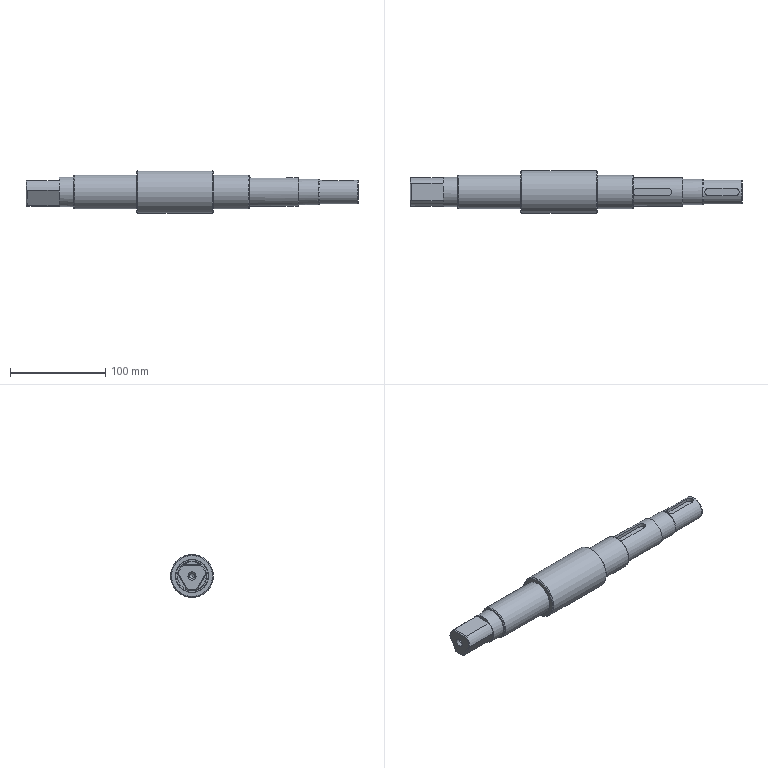Part | 1 solid | 59 faces | box 348.4 x 45 x 45 mm | volume 325259 mm3 | plane 26 | cylinder 19 | cone 14 | commonest cylinder face diameters 30 x5 8 x4 5 x3 35 x2 4 x1 25 x1
STEP:
#1=CARTESIAN_POINT('',(-139.2,8.889,-10.5));
#2=VERTEX_POINT('',#1);
#3=CARTESIAN_POINT('',(-139.2,-8.889,-10.5));
#4=VERTEX_POINT('',#3);
#5=CARTESIAN_POINT('',(-139.2,9.,-10.5));
#6=DIRECTION('',(0.,-1.,0.));
#7=VECTOR('',#6,1000.);
#8=LINE('',#5,#7);
#9=EDGE_CURVE('',#2,#4,#8,.T.);
#10=ORIENTED_EDGE('',*,*,#9,.T.);
#11=CARTESIAN_POINT('',(-139.2,0.,-22.5));
#12=DIRECTION('',(1.,0.,0.));
#13=DIRECTION('',(0.,1.,0.));
#14=AXIS2_PLACEMENT_3D('',#11,#12,#13);
#15=CIRCLE('',#14,14.934);
#16=EDGE_CURVE('',#4,#2,#15,.F.);
#17=ORIENTED_EDGE('',*,*,#16,.T.);
#18=EDGE_LOOP('',(#10,#17));
#19=FACE_BOUND('',#18,.T.);
#20=CARTESIAN_POINT('',(-139.2,0.,-7.1));
#21=DIRECTION('',(1.,0.,0.));
#22=DIRECTION('',(0.,1.,0.));
#23=AXIS2_PLACEMENT_3D('',#20,#21,#22);
#24=PLANE('',#23);
#25=ADVANCED_FACE('',(#19),#24,.F.);
#26=CARTESIAN_POINT('',(-139.2,5.892,-36.294));
#27=VERTEX_POINT('',#26);
#28=CARTESIAN_POINT('',(-139.2,14.892,-20.706));
#29=VERTEX_POINT('',#28);
#30=CARTESIAN_POINT('',(-139.2,5.892,-36.294));
#31=DIRECTION('',(0.,0.5,0.866));
#32=VECTOR('',#31,1000.);
#33=LINE('',#30,#32);
#34=EDGE_CURVE('',#27,#29,#33,.T.);
#35=ORIENTED_EDGE('',*,*,#34,.T.);
#36=CARTESIAN_POINT('',(-139.2,9.,-10.5));
#37=VERTEX_POINT('',#36);
#38=CARTESIAN_POINT('',(-139.2,0.,-22.5));
#39=DIRECTION('',(1.,0.,0.));
#40=DIRECTION('',(0.,0.,-1.));
#41=AXIS2_PLACEMENT_3D('',#38,#39,#40);
#42=CIRCLE('',#41,15.);
#43=EDGE_CURVE('',#37,#29,#42,.F.);
#44=ORIENTED_EDGE('',*,*,#43,.F.);
#45=CARTESIAN_POINT('',(-139.2,9.,-10.5));
#46=DIRECTION('',(0.,-1.,0.));
#47=VECTOR('',#46,1000.);
#48=LINE('',#45,#47);
#49=EDGE_CURVE('',#2,#37,#48,.F.);
#50=ORIENTED_EDGE('',*,*,#49,.F.);
#51=ORIENTED_EDGE('',*,*,#16,.F.);
#52=CARTESIAN_POINT('',(-139.2,-9.,-10.5));
#53=VERTEX_POINT('',#52);
#54=CARTESIAN_POINT('',(-139.2,9.,-10.5));
#55=DIRECTION('',(0.,-1.,0.));
#56=VECTOR('',#55,1000.);
#57=LINE('',#54,#56);
#58=EDGE_CURVE('',#53,#4,#57,.F.);
#59=ORIENTED_EDGE('',*,*,#58,.F.);
#60=CARTESIAN_POINT('',(-139.2,-14.892,-20.706));
#61=VERTEX_POINT('',#60);
#62=CARTESIAN_POINT('',(-139.2,0.,-22.5));
#63=DIRECTION('',(1.,0.,0.));
#64=DIRECTION('',(0.,0.,-1.));
#65=AXIS2_PLACEMENT_3D('',#62,#63,#64);
#66=CIRCLE('',#65,15.);
#67=EDGE_CURVE('',#61,#53,#66,.F.);
#68=ORIENTED_EDGE('',*,*,#67,.F.);
#69=CARTESIAN_POINT('',(-139.2,-14.837,-20.802));
#70=VERTEX_POINT('',#69);
#71=CARTESIAN_POINT('',(-139.2,-14.892,-20.706));
#72=DIRECTION('',(0.,0.5,-0.866));
#73=VECTOR('',#72,1000.);
#74=LINE('',#71,#73);
#75=EDGE_CURVE('',#70,#61,#74,.F.);
#76=ORIENTED_EDGE('',*,*,#75,.F.);
#77=CARTESIAN_POINT('',(-139.2,-5.948,-36.198));
#78=VERTEX_POINT('',#77);
#79=CARTESIAN_POINT('',(-139.2,0.,-22.5));
#80=DIRECTION('',(1.,0.,0.));
#81=DIRECTION('',(0.,1.,0.));
#82=AXIS2_PLACEMENT_3D('',#79,#80,#81);
#83=CIRCLE('',#82,14.934);
#84=EDGE_CURVE('',#78,#70,#83,.F.);
#85=ORIENTED_EDGE('',*,*,#84,.F.);
#86=CARTESIAN_POINT('',(-139.2,-5.892,-36.294));
#87=VERTEX_POINT('',#86);
#88=CARTESIAN_POINT('',(-139.2,-14.892,-20.706));
#89=DIRECTION('',(0.,0.5,-0.866));
#90=VECTOR('',#89,1000.);
#91=LINE('',#88,#90);
#92=EDGE_CURVE('',#87,#78,#91,.F.);
#93=ORIENTED_EDGE('',*,*,#92,.F.);
#94=CARTESIAN_POINT('',(-139.2,0.,-22.5));
#95=DIRECTION('',(1.,0.,0.));
#96=DIRECTION('',(0.,0.,-1.));
#97=AXIS2_PLACEMENT_3D('',#94,#95,#96);
#98=CIRCLE('',#97,15.);
#99=EDGE_CURVE('',#27,#87,#98,.F.);
#100=ORIENTED_EDGE('',*,*,#99,.F.);
#101=EDGE_LOOP('',(#35,#44,#50,#51,#59,#68,#76,#85,#93,#100));
#102=FACE_BOUND('',#101,.T.);
#103=CARTESIAN_POINT('',(-139.2,0.,-37.9));
#104=VERTEX_POINT('',#103);
#105=CARTESIAN_POINT('',(-139.2,0.,-22.5));
#106=DIRECTION('',(1.,0.,0.));
#107=DIRECTION('',(0.,0.,-1.));
#108=AXIS2_PLACEMENT_3D('',#105,#106,#107);
#109=CIRCLE('',#108,15.4);
#110=EDGE_CURVE('',#104,#104,#109,.T.);
#111=ORIENTED_EDGE('',*,*,#110,.F.);
#112=EDGE_LOOP('',(#111));
#113=FACE_BOUND('',#112,.T.);
#114=CARTESIAN_POINT('',(-139.2,0.,-7.1));
#115=DIRECTION('',(1.,0.,0.));
#116=DIRECTION('',(0.,1.,0.));
#117=AXIS2_PLACEMENT_3D('',#114,#115,#116);
#118=PLANE('',#117);
#119=ADVANCED_FACE('',(#102,#113),#118,.F.);
#120=CARTESIAN_POINT('',(-173.2,-9.303,-10.733));
#121=VERTEX_POINT('',#120);
#122=CARTESIAN_POINT('',(-173.2,-14.842,-20.327));
#123=VERTEX_POINT('',#122);
#124=CARTESIAN_POINT('',(-173.2,0.,-22.5));
#125=DIRECTION('',(1.,0.,0.));
#126=DIRECTION('',(0.,1.,0.));
#127=AXIS2_PLACEMENT_3D('',#124,#125,#126);
#128=CIRCLE('',#127,15.);
#129=EDGE_CURVE('',#121,#123,#128,.T.);
#130=ORIENTED_EDGE('',*,*,#129,.T.);
#131=CARTESIAN_POINT('',(-172.7,-14.892,-20.706));
#132=VERTEX_POINT('',#131);
#133=CARTESIAN_POINT('',(-198.434,0.,-22.5));
#134=DIRECTION('',(0.4226,0.7849,0.4532));
#135=DIRECTION('',(-0.9063,0.366,0.2113));
#136=AXIS2_PLACEMENT_3D('',#133,#134,#135);
#137=ELLIPSE('',#136,35.493,15.);
#138=EDGE_CURVE('',#123,#132,#137,.T.);
#139=ORIENTED_EDGE('',*,*,#138,.T.);
#140=CARTESIAN_POINT('',(-120.952,-14.892,-20.706));
#141=DIRECTION('',(-1.,0.,0.));
#142=VECTOR('',#141,1000.);
#143=LINE('',#140,#142);
#144=EDGE_CURVE('',#61,#132,#143,.T.);
#145=ORIENTED_EDGE('',*,*,#144,.F.);
#146=ORIENTED_EDGE('',*,*,#67,.T.);
#147=CARTESIAN_POINT('',(-172.7,-9.,-10.5));
#148=VERTEX_POINT('',#147);
#149=CARTESIAN_POINT('',(-120.952,-9.,-10.5));
#150=DIRECTION('',(-1.,0.,0.));
#151=VECTOR('',#150,1000.);
#152=LINE('',#149,#151);
#153=EDGE_CURVE('',#53,#148,#152,.T.);
#154=ORIENTED_EDGE('',*,*,#153,.T.);
#155=CARTESIAN_POINT('',(-198.434,0.,-22.5));
#156=DIRECTION('',(0.4226,0.,-0.9063));
#157=DIRECTION('',(-0.9063,0.,-0.4226));
#158=AXIS2_PLACEMENT_3D('',#155,#156,#157);
#159=ELLIPSE('',#158,35.493,15.);
#160=EDGE_CURVE('',#148,#121,#159,.T.);
#161=ORIENTED_EDGE('',*,*,#160,.T.);
#162=EDGE_LOOP('',(#130,#139,#145,#146,#154,#161));
#163=FACE_BOUND('',#162,.T.);
#164=CARTESIAN_POINT('',(-174.2,0.,-22.5));
#165=DIRECTION('',(-1.,0.,0.));
#166=DIRECTION('',(0.,-1.,0.));
#167=AXIS2_PLACEMENT_3D('',#164,#165,#166);
#168=CYLINDRICAL_SURFACE('',#167,15.);
#169=ADVANCED_FACE('',(#163),#168,.T.);
#170=CARTESIAN_POINT('',(-172.7,-5.892,-36.294));
#171=VERTEX_POINT('',#170);
#172=CARTESIAN_POINT('',(-120.952,-5.892,-36.294));
#173=DIRECTION('',(-1.,0.,0.));
#174=VECTOR('',#173,1000.);
#175=LINE('',#172,#174);
#176=EDGE_CURVE('',#87,#171,#175,.T.);
#177=ORIENTED_EDGE('',*,*,#176,.T.);
#178=CARTESIAN_POINT('',(-173.2,-5.539,-36.44));
#179=VERTEX_POINT('',#178);
#180=CARTESIAN_POINT('',(-198.434,0.,-22.5));
#181=DIRECTION('',(0.4226,0.7849,0.4532));
#182=DIRECTION('',(-0.9063,0.366,0.2113));
#183=AXIS2_PLACEMENT_3D('',#180,#181,#182);
#184=ELLIPSE('',#183,35.493,15.);
#185=EDGE_CURVE('',#171,#179,#184,.T.);
#186=ORIENTED_EDGE('',*,*,#185,.T.);
#187=CARTESIAN_POINT('',(-173.2,5.539,-36.44));
#188=VERTEX_POINT('',#187);
#189=CARTESIAN_POINT('',(-173.2,0.,-22.5));
#190=DIRECTION('',(1.,0.,0.));
#191=DIRECTION('',(0.,1.,0.));
#192=AXIS2_PLACEMENT_3D('',#189,#190,#191);
#193=CIRCLE('',#192,15.);
#194=EDGE_CURVE('',#179,#188,#193,.T.);
#195=ORIENTED_EDGE('',*,*,#194,.T.);
#196=CARTESIAN_POINT('',(-172.7,5.892,-36.294));
#197=VERTEX_POINT('',#196);
#198=CARTESIAN_POINT('',(-198.434,0.,-22.5));
#199=DIRECTION('',(0.4226,-0.7849,0.4532));
#200=DIRECTION('',(-0.9063,-0.366,0.2113));
#201=AXIS2_PLACEMENT_3D('',#198,#199,#200);
#202=ELLIPSE('',#201,35.493,15.);
#203=EDGE_CURVE('',#188,#197,#202,.T.);
#204=ORIENTED_EDGE('',*,*,#203,.T.);
#205=CARTESIAN_POINT('',(-120.952,5.892,-36.294));
#206=DIRECTION('',(-1.,0.,0.));
#207=VECTOR('',#206,1000.);
#208=LINE('',#205,#207);
#209=EDGE_CURVE('',#27,#197,#208,.T.);
#210=ORIENTED_EDGE('',*,*,#209,.F.);
#211=ORIENTED_EDGE('',*,*,#99,.T.);
#212=EDGE_LOOP('',(#177,#186,#195,#204,#210,#211));
#213=FACE_BOUND('',#212,.T.);
#214=CARTESIAN_POINT('',(-174.2,0.,-22.5));
#215=DIRECTION('',(-1.,0.,0.));
#216=DIRECTION('',(0.,-1.,0.));
#217=AXIS2_PLACEMENT_3D('',#214,#215,#216);
#218=CYLINDRICAL_SURFACE('',#217,15.);
#219=ADVANCED_FACE('',(#213),#218,.T.);
#220=CARTESIAN_POINT('',(-173.2,14.842,-20.327));
#221=VERTEX_POINT('',#220);
#222=CARTESIAN_POINT('',(-173.2,9.303,-10.733));
#223=VERTEX_POINT('',#222);
#224=CARTESIAN_POINT('',(-173.2,0.,-22.5));
#225=DIRECTION('',(1.,0.,0.));
#226=DIRECTION('',(0.,1.,0.));
#227=AXIS2_PLACEMENT_3D('',#224,#225,#226);
#228=CIRCLE('',#227,15.);
#229=EDGE_CURVE('',#221,#223,#228,.T.);
#230=ORIENTED_EDGE('',*,*,#229,.F.);
#231=CARTESIAN_POINT('',(-174.2,14.356,-20.235));
#232=VERTEX_POINT('',#231);
#233=CARTESIAN_POINT('',(-173.2,14.842,-20.327));
#234=CARTESIAN_POINT('',(-173.533,14.68,-20.296));
#235=CARTESIAN_POINT('',(-173.867,14.518,-20.266));
#236=CARTESIAN_POINT('',(-174.2,14.356,-20.235));
#237=B_SPLINE_CURVE_WITH_KNOTS('',3,(#233,#234,#235,#236),.UNSPECIFIED.,.F.,.F.,(4,4),(0.,0.001115),.UNSPECIFIED.);
#238=EDGE_CURVE('',#221,#232,#237,.T.);
#239=ORIENTED_EDGE('',*,*,#238,.T.);
#240=CARTESIAN_POINT('',(-174.2,9.139,-11.199));
#241=VERTEX_POINT('',#240);
#242=CARTESIAN_POINT('',(-174.2,0.,-22.5));
#243=DIRECTION('',(1.,0.,0.));
#244=DIRECTION('',(0.,1.,0.));
#245=AXIS2_PLACEMENT_3D('',#242,#243,#244);
#246=CIRCLE('',#245,14.534);
#247=EDGE_CURVE('',#241,#232,#246,.F.);
#248=ORIENTED_EDGE('',*,*,#247,.F.);
#249=CARTESIAN_POINT('',(-174.2,9.139,-11.199));
#250=CARTESIAN_POINT('',(-173.867,9.194,-11.044));
#251=CARTESIAN_POINT('',(-173.533,9.249,-10.889));
#252=CARTESIAN_POINT('',(-173.2,9.303,-10.733));
#253=B_SPLINE_CURVE_WITH_KNOTS('',3,(#249,#250,#251,#252),.UNSPECIFIED.,.F.,.F.,(4,4),(0.,0.001115),.UNSPECIFIED.);
#254=EDGE_CURVE('',#241,#223,#253,.T.);
#255=ORIENTED_EDGE('',*,*,#254,.T.);
#256=EDGE_LOOP('',(#230,#239,#248,#255));
#257=FACE_BOUND('',#256,.T.);
#258=CARTESIAN_POINT('',(-174.2,0.,-22.5));
#259=DIRECTION('',(1.,0.,0.));
#260=DIRECTION('',(0.,1.,0.));
#261=AXIS2_PLACEMENT_3D('',#258,#259,#260);
#262=CONICAL_SURFACE('',#261,14.534,0.4363);
#263=ADVANCED_FACE('',(#257),#262,.T.);
#264=CARTESIAN_POINT('',(-174.2,-14.356,-20.235));
#265=VERTEX_POINT('',#264);
#266=CARTESIAN_POINT('',(-174.2,-9.139,-11.199));
#267=VERTEX_POINT('',#266);
#268=CARTESIAN_POINT('',(-174.2,0.,-22.5));
#269=DIRECTION('',(1.,0.,0.));
#270=DIRECTION('',(0.,1.,0.));
#271=AXIS2_PLACEMENT_3D('',#268,#269,#270);
#272=CIRCLE('',#271,14.534);
#273=EDGE_CURVE('',#265,#267,#272,.F.);
#274=ORIENTED_EDGE('',*,*,#273,.F.);
#275=CARTESIAN_POINT('',(-174.2,-14.356,-20.235));
#276=CARTESIAN_POINT('',(-173.867,-14.518,-20.266));
#277=CARTESIAN_POINT('',(-173.533,-14.68,-20.296));
#278=CARTESIAN_POINT('',(-173.2,-14.842,-20.327));
#279=B_SPLINE_CURVE_WITH_KNOTS('',3,(#275,#276,#277,#278),.UNSPECIFIED.,.F.,.F.,(4,4),(0.,0.001115),.UNSPECIFIED.);
#280=EDGE_CURVE('',#265,#123,#279,.T.);
#281=ORIENTED_EDGE('',*,*,#280,.T.);
#282=ORIENTED_EDGE('',*,*,#129,.F.);
#283=CARTESIAN_POINT('',(-173.2,-9.303,-10.733));
#284=CARTESIAN_POINT('',(-173.533,-9.249,-10.889));
#285=CARTESIAN_POINT('',(-173.867,-9.194,-11.044));
#286=CARTESIAN_POINT('',(-174.2,-9.139,-11.199));
#287=B_SPLINE_CURVE_WITH_KNOTS('',3,(#283,#284,#285,#286),.UNSPECIFIED.,.F.,.F.,(4,4),(0.,0.001115),.UNSPECIFIED.);
#288=EDGE_CURVE('',#121,#267,#287,.T.);
#289=ORIENTED_EDGE('',*,*,#288,.T.);
#290=EDGE_LOOP('',(#274,#281,#282,#289));
#291=FACE_BOUND('',#290,.T.);
#292=CARTESIAN_POINT('',(-174.2,0.,-22.5));
#293=DIRECTION('',(1.,0.,0.));
#294=DIRECTION('',(0.,1.,0.));
#295=AXIS2_PLACEMENT_3D('',#292,#293,#294);
#296=CONICAL_SURFACE('',#295,14.534,0.4363);
#297=ADVANCED_FACE('',(#291),#296,.T.);
#298=CARTESIAN_POINT('',(134.2,-12.5,-22.5));
#299=VERTEX_POINT('',#298);
#300=CARTESIAN_POINT('',(134.2,0.,-22.5));
#301=DIRECTION('',(-1.,0.,0.));
#302=DIRECTION('',(0.,-1.,0.));
#303=AXIS2_PLACEMENT_3D('',#300,#301,#302);
#304=CIRCLE('',#303,12.5);
#305=EDGE_CURVE('',#299,#299,#304,.T.);
#306=ORIENTED_EDGE('',*,*,#305,.F.);
#307=EDGE_LOOP('',(#306));
#308=FACE_BOUND('',#307,.T.);
#309=CARTESIAN_POINT('',(173.2,-12.5,-22.5));
#310=VERTEX_POINT('',#309);
#311=CARTESIAN_POINT('',(173.2,0.,-22.5));
#312=DIRECTION('',(-1.,0.,0.));
#313=DIRECTION('',(0.,-1.,0.));
#314=AXIS2_PLACEMENT_3D('',#311,#312,#313);
#315=CIRCLE('',#314,12.5);
#316=EDGE_CURVE('',#310,#310,#315,.T.);
#317=ORIENTED_EDGE('',*,*,#316,.T.);
#318=EDGE_LOOP('',(#317));
#319=FACE_BOUND('',#318,.T.);
#320=CARTESIAN_POINT('',(139.2,-4.,-10.657));
#321=VERTEX_POINT('',#320);
#322=CARTESIAN_POINT('',(167.2,-4.,-10.657));
#323=VERTEX_POINT('',#322);
#324=CARTESIAN_POINT('',(-174.2,-4.,-10.657));
#325=DIRECTION('',(-1.,0.,0.));
#326=VECTOR('',#325,1000.);
#327=LINE('',#324,#326);
#328=EDGE_CURVE('',#321,#323,#327,.F.);
#329=ORIENTED_EDGE('',*,*,#328,.F.);
#330=CARTESIAN_POINT('',(139.2,4.,-10.657));
#331=VERTEX_POINT('',#330);
#332=CARTESIAN_POINT('',(139.2,4.,-10.657));
#333=CARTESIAN_POINT('',(138.136,4.,-10.657));
#334=CARTESIAN_POINT('',(136.076,3.133,-10.32));
#335=CARTESIAN_POINT('',(134.763,0.006695,-9.84));
#336=CARTESIAN_POINT('',(136.074,-3.135,-10.319));
#337=CARTESIAN_POINT('',(138.136,-4.,-10.657));
#338=CARTESIAN_POINT('',(139.2,-4.,-10.657));
#339=B_SPLINE_CURVE_WITH_KNOTS('',3,(#332,#333,#334,#335,#336,#337,#338),.UNSPECIFIED.,.F.,.F.,(4,1,1,1,4),(0.,0.003146,0.006292,0.009438,0.01258),.UNSPECIFIED.);
#340=EDGE_CURVE('',#331,#321,#339,.T.);
#341=ORIENTED_EDGE('',*,*,#340,.F.);
#342=CARTESIAN_POINT('',(167.2,4.,-10.657));
#343=VERTEX_POINT('',#342);
#344=CARTESIAN_POINT('',(-174.2,4.,-10.657));
#345=DIRECTION('',(-1.,0.,0.));
#346=VECTOR('',#345,1000.);
#347=LINE('',#344,#346);
#348=EDGE_CURVE('',#331,#343,#347,.F.);
#349=ORIENTED_EDGE('',*,*,#348,.T.);
#350=CARTESIAN_POINT('',(167.2,-4.,-10.657));
#351=CARTESIAN_POINT('',(168.264,-4.,-10.657));
#352=CARTESIAN_POINT('',(170.324,-3.133,-10.32));
#353=CARTESIAN_POINT('',(171.637,-0.006695,-9.84));
#354=CARTESIAN_POINT('',(170.326,3.135,-10.319));
#355=CARTESIAN_POINT('',(168.264,4.,-10.657));
#356=CARTESIAN_POINT('',(167.2,4.,-10.657));
#357=B_SPLINE_CURVE_WITH_KNOTS('',3,(#350,#351,#352,#353,#354,#355,#356),.UNSPECIFIED.,.F.,.F.,(4,1,1,1,4),(0.,0.003146,0.006292,0.009438,0.01258),.UNSPECIFIED.);
#358=EDGE_CURVE('',#323,#343,#357,.T.);
#359=ORIENTED_EDGE('',*,*,#358,.F.);
#360=EDGE_LOOP('',(#329,#341,#349,#359));
#361=FACE_BOUND('',#360,.T.);
#362=CARTESIAN_POINT('',(-174.2,0.,-22.5));
#363=DIRECTION('',(-1.,0.,0.));
#364=DIRECTION('',(0.,-1.,0.));
#365=AXIS2_PLACEMENT_3D('',#362,#363,#364);
#366=CYLINDRICAL_SURFACE('',#365,12.5);
#367=ADVANCED_FACE('',(#308,#319,#361),#366,.T.);
#368=CARTESIAN_POINT('',(102.2,-2.5,-37.29));
#369=VERTEX_POINT('',#368);
#370=CARTESIAN_POINT('',(111.623,-2.5,-37.29));
#371=VERTEX_POINT('',#370);
#372=CARTESIAN_POINT('',(-174.2,-2.5,-37.29));
#373=DIRECTION('',(-1.,0.,0.));
#374=VECTOR('',#373,1000.);
#375=LINE('',#372,#374);
#376=EDGE_CURVE('',#369,#371,#375,.F.);
#377=ORIENTED_EDGE('',*,*,#376,.T.);
#378=CARTESIAN_POINT('',(111.623,2.5,-37.29));
#379=VERTEX_POINT('',#378);
#380=CARTESIAN_POINT('',(111.623,0.,-22.5));
#381=DIRECTION('',(-1.,0.,0.));
#382=DIRECTION('',(0.,-1.,0.));
#383=AXIS2_PLACEMENT_3D('',#380,#381,#382);
#384=CIRCLE('',#383,15.);
#385=EDGE_CURVE('',#371,#379,#384,.T.);
#386=ORIENTED_EDGE('',*,*,#385,.T.);
#387=CARTESIAN_POINT('',(102.2,2.5,-37.29));
#388=VERTEX_POINT('',#387);
#389=CARTESIAN_POINT('',(-174.2,2.5,-37.29));
#390=DIRECTION('',(-1.,0.,0.));
#391=VECTOR('',#390,1000.);
#392=LINE('',#389,#391);
#393=EDGE_CURVE('',#379,#388,#392,.T.);
#394=ORIENTED_EDGE('',*,*,#393,.T.);
#395=CARTESIAN_POINT('',(102.2,2.5,-37.29));
#396=CARTESIAN_POINT('',(101.538,2.5,-37.29));
#397=CARTESIAN_POINT('',(100.245,1.958,-37.396));
#398=CARTESIAN_POINT('',(99.428,0.002866,-37.552));
#399=CARTESIAN_POINT('',(100.243,-1.958,-37.396));
#400=CARTESIAN_POINT('',(101.538,-2.5,-37.29));
#401=CARTESIAN_POINT('',(102.2,-2.5,-37.29));
#402=B_SPLINE_CURVE_WITH_KNOTS('',3,(#395,#396,#397,#398,#399,#400,#401),.UNSPECIFIED.,.F.,.F.,(4,1,1,1,4),(0.,0.001957,0.003914,0.005871,0.007828),.UNSPECIFIED.);
#403=EDGE_CURVE('',#388,#369,#402,.T.);
#404=ORIENTED_EDGE('',*,*,#403,.T.);
#405=EDGE_LOOP('',(#377,#386,#394,#404));
#406=FACE_BOUND('',#405,.T.);
#407=CARTESIAN_POINT('',(64.2,-4.,-8.043));
#408=VERTEX_POINT('',#407);
#409=CARTESIAN_POINT('',(96.2,-4.,-8.043));
#410=VERTEX_POINT('',#409);
#411=CARTESIAN_POINT('',(-174.2,-4.,-8.043));
#412=DIRECTION('',(-1.,0.,0.));
#413=VECTOR('',#412,1000.);
#414=LINE('',#411,#413);
#415=EDGE_CURVE('',#408,#410,#414,.F.);
#416=ORIENTED_EDGE('',*,*,#415,.F.);
#417=CARTESIAN_POINT('',(60.2,0.,-7.5));
#418=VERTEX_POINT('',#417);
#419=CARTESIAN_POINT('',(60.2,0.,-7.5));
#420=CARTESIAN_POINT('',(60.2,-1.048,-7.5));
#421=CARTESIAN_POINT('',(61.074,-3.133,-7.767));
#422=CARTESIAN_POINT('',(63.139,-4.,-8.043));
#423=CARTESIAN_POINT('',(64.2,-4.,-8.043));
#424=B_SPLINE_CURVE_WITH_KNOTS('',3,(#419,#420,#421,#422,#423),.UNSPECIFIED.,.F.,.F.,(4,1,4),(0.006283,0.009421,0.01256),.UNSPECIFIED.);
#425=EDGE_CURVE('',#418,#408,#424,.T.);
#426=ORIENTED_EDGE('',*,*,#425,.F.);
#427=CARTESIAN_POINT('',(60.2,0.,-22.5));
#428=DIRECTION('',(-1.,0.,0.));
#429=DIRECTION('',(0.,-1.,0.));
#430=AXIS2_PLACEMENT_3D('',#427,#428,#429);
#431=CIRCLE('',#430,15.);
#432=EDGE_CURVE('',#418,#418,#431,.T.);
#433=ORIENTED_EDGE('',*,*,#432,.F.);
#434=CARTESIAN_POINT('',(64.2,4.,-8.043));
#435=VERTEX_POINT('',#434);
#436=CARTESIAN_POINT('',(64.2,4.,-8.043));
#437=CARTESIAN_POINT('',(63.137,4.,-8.043));
#438=CARTESIAN_POINT('',(61.072,3.13,-7.766));
#439=CARTESIAN_POINT('',(60.2,1.049,-7.5));
#440=CARTESIAN_POINT('',(60.2,0.,-7.5));
#441=B_SPLINE_CURVE_WITH_KNOTS('',3,(#436,#437,#438,#439,#440),.UNSPECIFIED.,.F.,.F.,(4,1,4),(0.,0.003142,0.006283),.UNSPECIFIED.);
#442=EDGE_CURVE('',#435,#418,#441,.T.);
#443=ORIENTED_EDGE('',*,*,#442,.F.);
#444=CARTESIAN_POINT('',(96.2,4.,-8.043));
#445=VERTEX_POINT('',#444);
#446=CARTESIAN_POINT('',(-174.2,4.,-8.043));
#447=DIRECTION('',(-1.,0.,0.));
#448=VECTOR('',#447,1000.);
#449=LINE('',#446,#448);
#450=EDGE_CURVE('',#435,#445,#449,.F.);
#451=ORIENTED_EDGE('',*,*,#450,.T.);
#452=CARTESIAN_POINT('',(96.2,-4.,-8.043));
#453=CARTESIAN_POINT('',(97.262,-4.,-8.043));
#454=CARTESIAN_POINT('',(99.326,-3.133,-7.767));
#455=CARTESIAN_POINT('',(100.637,-0.005849,-7.367));
#456=CARTESIAN_POINT('',(99.328,3.134,-7.766));
#457=CARTESIAN_POINT('',(97.262,4.,-8.043));
#458=CARTESIAN_POINT('',(96.2,4.,-8.043));
#459=B_SPLINE_CURVE_WITH_KNOTS('',3,(#452,#453,#454,#455,#456,#457,#458),.UNSPECIFIED.,.F.,.F.,(4,1,1,1,4),(0.,0.00314,0.006279,0.009419,0.01256),.UNSPECIFIED.);
#460=EDGE_CURVE('',#410,#445,#459,.T.);
#461=ORIENTED_EDGE('',*,*,#460,.F.);
#462=EDGE_LOOP('',(#416,#426,#433,#443,#451,#461));
#463=FACE_BOUND('',#462,.T.);
#464=CARTESIAN_POINT('',(-174.2,0.,-22.5));
#465=DIRECTION('',(-1.,0.,0.));
#466=DIRECTION('',(0.,-1.,0.));
#467=AXIS2_PLACEMENT_3D('',#464,#465,#466);
#468=CYLINDRICAL_SURFACE('',#467,15.);
#469=ADVANCED_FACE('',(#406,#463),#468,.T.);
#470=CARTESIAN_POINT('',(-174.2,-4.25,-22.5));
#471=VERTEX_POINT('',#470);
#472=CARTESIAN_POINT('',(-174.2,0.,-22.5));
#473=DIRECTION('',(-1.,0.,0.));
#474=DIRECTION('',(0.,-1.,0.));
#475=AXIS2_PLACEMENT_3D('',#472,#473,#474);
#476=CIRCLE('',#475,4.25);
#477=EDGE_CURVE('',#471,#471,#476,.T.);
#478=ORIENTED_EDGE('',*,*,#477,.F.);
#479=EDGE_LOOP('',(#478));
#480=FACE_BOUND('',#479,.T.);
#481=CARTESIAN_POINT('',(-174.2,5.217,-36.065));
#482=VERTEX_POINT('',#481);
#483=CARTESIAN_POINT('',(-174.2,-5.217,-36.065));
#484=VERTEX_POINT('',#483);
#485=CARTESIAN_POINT('',(-174.2,0.,-22.5));
#486=DIRECTION('',(1.,0.,0.));
#487=DIRECTION('',(0.,1.,0.));
#488=AXIS2_PLACEMENT_3D('',#485,#486,#487);
#489=CIRCLE('',#488,14.534);
#490=EDGE_CURVE('',#482,#484,#489,.F.);
#491=ORIENTED_EDGE('',*,*,#490,.T.);
#492=CARTESIAN_POINT('',(-174.2,-9.787,-28.15));
#493=DIRECTION('',(0.,-0.5,0.866));
#494=VECTOR('',#493,1000.);
#495=LINE('',#492,#494);
#496=EDGE_CURVE('',#484,#265,#495,.T.);
#497=ORIENTED_EDGE('',*,*,#496,.T.);
#498=ORIENTED_EDGE('',*,*,#273,.T.);
#499=CARTESIAN_POINT('',(-174.2,0.,-11.199));
#500=DIRECTION('',(0.,1.,0.));
#501=VECTOR('',#500,1000.);
#502=LINE('',#499,#501);
#503=EDGE_CURVE('',#267,#241,#502,.T.);
#504=ORIENTED_EDGE('',*,*,#503,.T.);
#505=ORIENTED_EDGE('',*,*,#247,.T.);
#506=CARTESIAN_POINT('',(-174.2,9.787,-28.15));
#507=DIRECTION('',(0.,-0.5,-0.866));
#508=VECTOR('',#507,1000.);
#509=LINE('',#506,#508);
#510=EDGE_CURVE('',#232,#482,#509,.T.);
#511=ORIENTED_EDGE('',*,*,#510,.T.);
#512=EDGE_LOOP('',(#491,#497,#498,#504,#505,#511));
#513=FACE_BOUND('',#512,.T.);
#514=CARTESIAN_POINT('',(-174.2,0.,-22.5));
#515=DIRECTION('',(1.,0.,0.));
#516=DIRECTION('',(0.,1.,0.));
#517=AXIS2_PLACEMENT_3D('',#514,#515,#516);
#518=PLANE('',#517);
#519=ADVANCED_FACE('',(#480,#513),#518,.F.);
#520=CARTESIAN_POINT('',(-172.7,14.892,-20.706));
#521=VERTEX_POINT('',#520);
#522=CARTESIAN_POINT('',(-120.952,14.892,-20.706));
#523=DIRECTION('',(-1.,0.,0.));
#524=VECTOR('',#523,1000.);
#525=LINE('',#522,#524);
#526=EDGE_CURVE('',#29,#521,#525,.T.);
#527=ORIENTED_EDGE('',*,*,#526,.T.);
#528=CARTESIAN_POINT('',(-198.434,0.,-22.5));
#529=DIRECTION('',(0.4226,-0.7849,0.4532));
#530=DIRECTION('',(-0.9063,-0.366,0.2113));
#531=AXIS2_PLACEMENT_3D('',#528,#529,#530);
#532=ELLIPSE('',#531,35.493,15.);
#533=EDGE_CURVE('',#521,#221,#532,.T.);
#534=ORIENTED_EDGE('',*,*,#533,.T.);
#535=ORIENTED_EDGE('',*,*,#229,.T.);
#536=CARTESIAN_POINT('',(-172.7,9.,-10.5));
#537=VERTEX_POINT('',#536);
#538=CARTESIAN_POINT('',(-198.434,0.,-22.5));
#539=DIRECTION('',(0.4226,0.,-0.9063));
#540=DIRECTION('',(-0.9063,0.,-0.4226));
#541=AXIS2_PLACEMENT_3D('',#538,#539,#540);
#542=ELLIPSE('',#541,35.493,15.);
#543=EDGE_CURVE('',#223,#537,#542,.T.);
#544=ORIENTED_EDGE('',*,*,#543,.T.);
#545=CARTESIAN_POINT('',(-120.952,9.,-10.5));
#546=DIRECTION('',(-1.,0.,0.));
#547=VECTOR('',#546,1000.);
#548=LINE('',#545,#547);
#549=EDGE_CURVE('',#37,#537,#548,.T.);
#550=ORIENTED_EDGE('',*,*,#549,.F.);
#551=ORIENTED_EDGE('',*,*,#43,.T.);
#552=EDGE_LOOP('',(#527,#534,#535,#544,#550,#551));
#553=FACE_BOUND('',#552,.T.);
#554=CARTESIAN_POINT('',(-174.2,0.,-22.5));
#555=DIRECTION('',(-1.,0.,0.));
#556=DIRECTION('',(0.,-1.,0.));
#557=AXIS2_PLACEMENT_3D('',#554,#555,#556);
#558=CYLINDRICAL_SURFACE('',#557,15.);
#559=ADVANCED_FACE('',(#553),#558,.T.);
#560=CARTESIAN_POINT('',(-139.2,-14.892,-20.706));
#561=DIRECTION('',(0.,0.5,-0.866));
#562=VECTOR('',#561,1000.);
#563=LINE('',#560,#562);
#564=EDGE_CURVE('',#70,#78,#563,.T.);
#565=ORIENTED_EDGE('',*,*,#564,.T.);
#566=ORIENTED_EDGE('',*,*,#84,.T.);
#567=EDGE_LOOP('',(#565,#566));
#568=FACE_BOUND('',#567,.T.);
#569=CARTESIAN_POINT('',(-139.2,0.,-7.1));
#570=DIRECTION('',(1.,0.,0.));
#571=DIRECTION('',(0.,1.,0.));
#572=AXIS2_PLACEMENT_3D('',#569,#570,#571);
#573=PLANE('',#572);
#574=ADVANCED_FACE('',(#568),#573,.F.);
#575=ORIENTED_EDGE('',*,*,#110,.T.);
#576=EDGE_LOOP('',(#575));
#577=FACE_BOUND('',#576,.T.);
#578=CARTESIAN_POINT('',(-124.2,-15.4,-22.5));
#579=VERTEX_POINT('',#578);
#580=CARTESIAN_POINT('',(-124.2,0.,-22.5));
#581=DIRECTION('',(-1.,0.,0.));
#582=DIRECTION('',(0.,-1.,0.));
#583=AXIS2_PLACEMENT_3D('',#580,#581,#582);
#584=CIRCLE('',#583,15.4);
#585=EDGE_CURVE('',#579,#579,#584,.T.);
#586=ORIENTED_EDGE('',*,*,#585,.T.);
#587=EDGE_LOOP('',(#586));
#588=FACE_BOUND('',#587,.T.);
#589=CARTESIAN_POINT('',(-174.2,0.,-22.5));
#590=DIRECTION('',(-1.,0.,0.));
#591=DIRECTION('',(0.,-1.,0.));
#592=AXIS2_PLACEMENT_3D('',#589,#590,#591);
#593=CYLINDRICAL_SURFACE('',#592,15.4);
#594=ADVANCED_FACE('',(#577,#588),#593,.T.);
#595=CARTESIAN_POINT('',(-124.2,17.034,-22.5));
#596=VERTEX_POINT('',#595);
#597=CARTESIAN_POINT('',(-124.2,0.,-22.5));
#598=DIRECTION('',(1.,0.,0.));
#599=DIRECTION('',(0.,1.,0.));
#600=AXIS2_PLACEMENT_3D('',#597,#598,#599);
#601=CIRCLE('',#600,17.034);
#602=EDGE_CURVE('',#596,#596,#601,.F.);
#603=ORIENTED_EDGE('',*,*,#602,.T.);
#604=EDGE_LOOP('',(#603));
#605=FACE_BOUND('',#604,.T.);
#606=ORIENTED_EDGE('',*,*,#585,.F.);
#607=EDGE_LOOP('',(#606));
#608=FACE_BOUND('',#607,.T.);
#609=CARTESIAN_POINT('',(-124.2,0.,-7.1));
#610=DIRECTION('',(1.,0.,0.));
#611=DIRECTION('',(0.,1.,0.));
#612=AXIS2_PLACEMENT_3D('',#609,#610,#611);
#613=PLANE('',#612);
#614=ADVANCED_FACE('',(#605,#608),#613,.F.);
#615=CARTESIAN_POINT('',(-123.2,17.5,-22.5));
#616=VERTEX_POINT('',#615);
#617=CARTESIAN_POINT('',(-123.2,0.,-22.5));
#618=DIRECTION('',(1.,0.,0.));
#619=DIRECTION('',(0.,1.,0.));
#620=AXIS2_PLACEMENT_3D('',#617,#618,#619);
#621=CIRCLE('',#620,17.5);
#622=EDGE_CURVE('',#616,#616,#621,.T.);
#623=ORIENTED_EDGE('',*,*,#622,.T.);
#624=EDGE_LOOP('',(#623));
#625=FACE_BOUND('',#624,.T.);
#626=CARTESIAN_POINT('',(-57.8,-17.5,-22.5));
#627=VERTEX_POINT('',#626);
#628=CARTESIAN_POINT('',(-57.8,0.,-22.5));
#629=DIRECTION('',(-1.,0.,0.));
#630=DIRECTION('',(0.,-1.,0.));
#631=AXIS2_PLACEMENT_3D('',#628,#629,#630);
#632=CIRCLE('',#631,17.5);
#633=EDGE_CURVE('',#627,#627,#632,.T.);
#634=ORIENTED_EDGE('',*,*,#633,.T.);
#635=EDGE_LOOP('',(#634));
#636=FACE_BOUND('',#635,.T.);
#637=CARTESIAN_POINT('',(-174.2,0.,-22.5));
#638=DIRECTION('',(-1.,0.,0.));
#639=DIRECTION('',(0.,-1.,0.));
#640=AXIS2_PLACEMENT_3D('',#637,#638,#639);
#641=CYLINDRICAL_SURFACE('',#640,17.5);
#642=ADVANCED_FACE('',(#625,#636),#641,.T.);
#643=CARTESIAN_POINT('',(-57.8,21.5,-22.5));
#644=VERTEX_POINT('',#643);
#645=CARTESIAN_POINT('',(-57.8,0.,-22.5));
#646=DIRECTION('',(1.,0.,0.));
#647=DIRECTION('',(0.,1.,0.));
#648=AXIS2_PLACEMENT_3D('',#645,#646,#647);
#649=CIRCLE('',#648,21.5);
#650=EDGE_CURVE('',#644,#644,#649,.F.);
#651=ORIENTED_EDGE('',*,*,#650,.T.);
#652=EDGE_LOOP('',(#651));
#653=FACE_BOUND('',#652,.T.);
#654=ORIENTED_EDGE('',*,*,#633,.F.);
#655=EDGE_LOOP('',(#654));
#656=FACE_BOUND('',#655,.T.);
#657=CARTESIAN_POINT('',(-57.8,0.,-5.));
#658=DIRECTION('',(1.,0.,0.));
#659=DIRECTION('',(0.,1.,0.));
#660=AXIS2_PLACEMENT_3D('',#657,#658,#659);
#661=PLANE('',#660);
#662=ADVANCED_FACE('',(#653,#656),#661,.F.);
#663=CARTESIAN_POINT('',(-56.8,22.5,-22.5));
#664=VERTEX_POINT('',#663);
#665=CARTESIAN_POINT('',(-56.8,0.,-22.5));
#666=DIRECTION('',(1.,0.,0.));
#667=DIRECTION('',(0.,1.,0.));
#668=AXIS2_PLACEMENT_3D('',#665,#666,#667);
#669=CIRCLE('',#668,22.5);
#670=EDGE_CURVE('',#664,#664,#669,.T.);
#671=ORIENTED_EDGE('',*,*,#670,.T.);
#672=EDGE_LOOP('',(#671));
#673=FACE_BOUND('',#672,.T.);
#674=CARTESIAN_POINT('',(21.2,-22.5,-22.5));
#675=VERTEX_POINT('',#674);
#676=CARTESIAN_POINT('',(21.2,0.,-22.5));
#677=DIRECTION('',(-1.,0.,0.));
#678=DIRECTION('',(0.,-1.,0.));
#679=AXIS2_PLACEMENT_3D('',#676,#677,#678);
#680=CIRCLE('',#679,22.5);
#681=EDGE_CURVE('',#675,#675,#680,.T.);
#682=ORIENTED_EDGE('',*,*,#681,.T.);
#683=EDGE_LOOP('',(#682));
#684=FACE_BOUND('',#683,.T.);
#685=CARTESIAN_POINT('',(-174.2,0.,-22.5));
#686=DIRECTION('',(-1.,0.,0.));
#687=DIRECTION('',(0.,-1.,0.));
#688=AXIS2_PLACEMENT_3D('',#685,#686,#687);
#689=CYLINDRICAL_SURFACE('',#688,22.5);
#690=ADVANCED_FACE('',(#673,#684),#689,.T.);
#691=CARTESIAN_POINT('',(22.2,-21.5,-22.5));
#692=VERTEX_POINT('',#691);
#693=CARTESIAN_POINT('',(22.2,0.,-22.5));
#694=DIRECTION('',(-1.,0.,0.));
#695=DIRECTION('',(0.,-1.,0.));
#696=AXIS2_PLACEMENT_3D('',#693,#694,#695);
#697=CIRCLE('',#696,21.5);
#698=EDGE_CURVE('',#692,#692,#697,.F.);
#699=ORIENTED_EDGE('',*,*,#698,.T.);
#700=EDGE_LOOP('',(#699));
#701=FACE_BOUND('',#700,.T.);
#702=CARTESIAN_POINT('',(22.2,-17.5,-22.5));
#703=VERTEX_POINT('',#702);
#704=CARTESIAN_POINT('',(22.2,0.,-22.5));
#705=DIRECTION('',(-1.,0.,0.));
#706=DIRECTION('',(0.,-1.,0.));
#707=AXIS2_PLACEMENT_3D('',#704,#705,#706);
#708=CIRCLE('',#707,17.5);
#709=EDGE_CURVE('',#703,#703,#708,.T.);
#710=ORIENTED_EDGE('',*,*,#709,.T.);
#711=EDGE_LOOP('',(#710));
#712=FACE_BOUND('',#711,.T.);
#713=CARTESIAN_POINT('',(22.2,0.,0.));
#714=DIRECTION('',(-1.,0.,0.));
#715=DIRECTION('',(0.,-1.,0.));
#716=AXIS2_PLACEMENT_3D('',#713,#714,#715);
#717=PLANE('',#716);
#718=ADVANCED_FACE('',(#701,#712),#717,.F.);
#719=CARTESIAN_POINT('',(59.2,-17.5,-22.5));
#720=VERTEX_POINT('',#719);
#721=CARTESIAN_POINT('',(59.2,0.,-22.5));
#722=DIRECTION('',(-1.,0.,0.));
#723=DIRECTION('',(0.,-1.,0.));
#724=AXIS2_PLACEMENT_3D('',#721,#722,#723);
#725=CIRCLE('',#724,17.5);
#726=EDGE_CURVE('',#720,#720,#725,.T.);
#727=ORIENTED_EDGE('',*,*,#726,.T.);
#728=EDGE_LOOP('',(#727));
#729=FACE_BOUND('',#728,.T.);
#730=ORIENTED_EDGE('',*,*,#709,.F.);
#731=EDGE_LOOP('',(#730));
#732=FACE_BOUND('',#731,.T.);
#733=CARTESIAN_POINT('',(-174.2,0.,-22.5));
#734=DIRECTION('',(-1.,0.,0.));
#735=DIRECTION('',(0.,-1.,0.));
#736=AXIS2_PLACEMENT_3D('',#733,#734,#735);
#737=CYLINDRICAL_SURFACE('',#736,17.5);
#738=ADVANCED_FACE('',(#729,#732),#737,.T.);
#739=CARTESIAN_POINT('',(60.2,-17.034,-22.5));
#740=VERTEX_POINT('',#739);
#741=CARTESIAN_POINT('',(60.2,0.,-22.5));
#742=DIRECTION('',(-1.,0.,0.));
#743=DIRECTION('',(0.,-1.,0.));
#744=AXIS2_PLACEMENT_3D('',#741,#742,#743);
#745=CIRCLE('',#744,17.034);
#746=EDGE_CURVE('',#740,#740,#745,.F.);
#747=ORIENTED_EDGE('',*,*,#746,.T.);
#748=EDGE_LOOP('',(#747));
#749=FACE_BOUND('',#748,.T.);
#750=ORIENTED_EDGE('',*,*,#432,.T.);
#751=EDGE_LOOP('',(#750));
#752=FACE_BOUND('',#751,.T.);
#753=CARTESIAN_POINT('',(60.2,0.,-5.));
#754=DIRECTION('',(-1.,0.,0.));
#755=DIRECTION('',(0.,-1.,0.));
#756=AXIS2_PLACEMENT_3D('',#753,#754,#755);
#757=PLANE('',#756);
#758=ADVANCED_FACE('',(#749,#752),#757,.F.);
#759=CARTESIAN_POINT('',(112.2,2.5,-36.275));
#760=VERTEX_POINT('',#759);
#761=CARTESIAN_POINT('',(112.2,2.5,-35.766));
#762=VERTEX_POINT('',#761);
#763=CARTESIAN_POINT('',(112.2,2.5,-44.5));
#764=DIRECTION('',(0.,0.,1.));
#765=VECTOR('',#764,1000.);
#766=LINE('',#763,#765);
#767=EDGE_CURVE('',#760,#762,#766,.T.);
#768=ORIENTED_EDGE('',*,*,#767,.F.);
#769=CARTESIAN_POINT('',(112.2,-2.5,-36.275));
#770=VERTEX_POINT('',#769);
#771=CARTESIAN_POINT('',(112.2,0.,-22.5));
#772=DIRECTION('',(-1.,0.,0.));
#773=DIRECTION('',(0.,-1.,0.));
#774=AXIS2_PLACEMENT_3D('',#771,#772,#773);
#775=CIRCLE('',#774,14.);
#776=EDGE_CURVE('',#760,#770,#775,.F.);
#777=ORIENTED_EDGE('',*,*,#776,.T.);
#778=CARTESIAN_POINT('',(112.2,-2.5,-35.766));
#779=VERTEX_POINT('',#778);
#780=CARTESIAN_POINT('',(112.2,-2.5,-44.5));
#781=DIRECTION('',(0.,0.,1.));
#782=VECTOR('',#781,1000.);
#783=LINE('',#780,#782);
#784=EDGE_CURVE('',#770,#779,#783,.T.);
#785=ORIENTED_EDGE('',*,*,#784,.T.);
#786=CARTESIAN_POINT('',(112.2,0.,-22.5));
#787=DIRECTION('',(-1.,0.,0.));
#788=DIRECTION('',(0.,-1.,0.));
#789=AXIS2_PLACEMENT_3D('',#786,#787,#788);
#790=CIRCLE('',#789,13.5);
#791=EDGE_CURVE('',#779,#762,#790,.T.);
#792=ORIENTED_EDGE('',*,*,#791,.T.);
#793=EDGE_LOOP('',(#768,#777,#785,#792));
#794=FACE_BOUND('',#793,.T.);
#795=CARTESIAN_POINT('',(112.2,0.,-7.5));
#796=DIRECTION('',(-1.,0.,0.));
#797=DIRECTION('',(0.,-1.,0.));
#798=AXIS2_PLACEMENT_3D('',#795,#796,#797);
#799=PLANE('',#798);
#800=ADVANCED_FACE('',(#794),#799,.F.);
#801=CARTESIAN_POINT('',(133.2,-13.5,-22.5));
#802=VERTEX_POINT('',#801);
#803=CARTESIAN_POINT('',(133.2,0.,-22.5));
#804=DIRECTION('',(-1.,0.,0.));
#805=DIRECTION('',(0.,-1.,0.));
#806=AXIS2_PLACEMENT_3D('',#803,#804,#805);
#807=CIRCLE('',#806,13.5);
#808=EDGE_CURVE('',#802,#802,#807,.T.);
#809=ORIENTED_EDGE('',*,*,#808,.T.);
#810=EDGE_LOOP('',(#809));
#811=FACE_BOUND('',#810,.T.);
#812=ORIENTED_EDGE('',*,*,#791,.F.);
#813=CARTESIAN_POINT('',(112.2,-2.5,-35.766));
#814=CARTESIAN_POINT('',(112.862,-2.5,-35.766));
#815=CARTESIAN_POINT('',(114.155,-1.958,-35.884));
#816=CARTESIAN_POINT('',(114.972,-0.00299,-36.058));
#817=CARTESIAN_POINT('',(114.156,1.958,-35.885));
#818=CARTESIAN_POINT('',(112.862,2.5,-35.766));
#819=CARTESIAN_POINT('',(112.2,2.5,-35.766));
#820=B_SPLINE_CURVE_WITH_KNOTS('',3,(#813,#814,#815,#816,#817,#818,#819),.UNSPECIFIED.,.F.,.F.,(4,1,1,1,4),(0.,0.001958,0.003916,0.005873,0.007831),.UNSPECIFIED.);
#821=EDGE_CURVE('',#779,#762,#820,.T.);
#822=ORIENTED_EDGE('',*,*,#821,.T.);
#823=EDGE_LOOP('',(#812,#822));
#824=FACE_BOUND('',#823,.T.);
#825=CARTESIAN_POINT('',(-174.2,0.,-22.5));
#826=DIRECTION('',(-1.,0.,0.));
#827=DIRECTION('',(0.,-1.,0.));
#828=AXIS2_PLACEMENT_3D('',#825,#826,#827);
#829=CYLINDRICAL_SURFACE('',#828,13.5);
#830=ADVANCED_FACE('',(#811,#824),#829,.T.);
#831=CARTESIAN_POINT('',(134.2,-13.034,-22.5));
#832=VERTEX_POINT('',#831);
#833=CARTESIAN_POINT('',(134.2,0.,-22.5));
#834=DIRECTION('',(-1.,0.,0.));
#835=DIRECTION('',(0.,-1.,0.));
#836=AXIS2_PLACEMENT_3D('',#833,#834,#835);
#837=CIRCLE('',#836,13.034);
#838=EDGE_CURVE('',#832,#832,#837,.F.);
#839=ORIENTED_EDGE('',*,*,#838,.T.);
#840=EDGE_LOOP('',(#839));
#841=FACE_BOUND('',#840,.T.);
#842=ORIENTED_EDGE('',*,*,#305,.T.);
#843=EDGE_LOOP('',(#842));
#844=FACE_BOUND('',#843,.T.);
#845=CARTESIAN_POINT('',(134.2,0.,-9.));
#846=DIRECTION('',(-1.,0.,0.));
#847=DIRECTION('',(0.,-1.,0.));
#848=AXIS2_PLACEMENT_3D('',#845,#846,#847);
#849=PLANE('',#848);
#850=ADVANCED_FACE('',(#841,#844),#849,.F.);
#851=CARTESIAN_POINT('',(174.2,4.25,-22.5));
#852=VERTEX_POINT('',#851);
#853=CARTESIAN_POINT('',(174.2,0.,-22.5));
#854=DIRECTION('',(1.,0.,0.));
#855=DIRECTION('',(0.,1.,0.));
#856=AXIS2_PLACEMENT_3D('',#853,#854,#855);
#857=CIRCLE('',#856,4.25);
#858=EDGE_CURVE('',#852,#852,#857,.T.);
#859=ORIENTED_EDGE('',*,*,#858,.F.);
#860=EDGE_LOOP('',(#859));
#861=FACE_BOUND('',#860,.T.);
#862=CARTESIAN_POINT('',(174.2,-12.034,-22.5));
#863=VERTEX_POINT('',#862);
#864=CARTESIAN_POINT('',(174.2,0.,-22.5));
#865=DIRECTION('',(-1.,0.,0.));
#866=DIRECTION('',(0.,-1.,0.));
#867=AXIS2_PLACEMENT_3D('',#864,#865,#866);
#868=CIRCLE('',#867,12.034);
#869=EDGE_CURVE('',#863,#863,#868,.F.);
#870=ORIENTED_EDGE('',*,*,#869,.T.);
#871=EDGE_LOOP('',(#870));
#872=FACE_BOUND('',#871,.T.);
#873=CARTESIAN_POINT('',(174.2,0.,-10.));
#874=DIRECTION('',(-1.,0.,0.));
#875=DIRECTION('',(0.,-1.,0.));
#876=AXIS2_PLACEMENT_3D('',#873,#874,#875);
#877=PLANE('',#876);
#878=ADVANCED_FACE('',(#861,#872),#877,.F.);
#879=ORIENTED_EDGE('',*,*,#415,.T.);
#880=CARTESIAN_POINT('',(96.2,-4.,-11.5));
#881=VERTEX_POINT('',#880);
#882=CARTESIAN_POINT('',(96.2,-4.,-1.5));
#883=DIRECTION('',(0.,0.,-1.));
#884=VECTOR('',#883,1000.);
#885=LINE('',#882,#884);
#886=EDGE_CURVE('',#410,#881,#885,.T.);
#887=ORIENTED_EDGE('',*,*,#886,.T.);
#888=CARTESIAN_POINT('',(64.2,-4.,-11.5));
#889=VERTEX_POINT('',#888);
#890=CARTESIAN_POINT('',(-174.2,-4.,-11.5));
#891=DIRECTION('',(1.,0.,0.));
#892=VECTOR('',#891,1000.);
#893=LINE('',#890,#892);
#894=EDGE_CURVE('',#889,#881,#893,.T.);
#895=ORIENTED_EDGE('',*,*,#894,.F.);
#896=CARTESIAN_POINT('',(64.2,-4.,-1.5));
#897=DIRECTION('',(0.,0.,-1.));
#898=VECTOR('',#897,1000.);
#899=LINE('',#896,#898);
#900=EDGE_CURVE('',#408,#889,#899,.T.);
#901=ORIENTED_EDGE('',*,*,#900,.F.);
#902=EDGE_LOOP('',(#879,#887,#895,#901));
#903=FACE_BOUND('',#902,.T.);
#904=CARTESIAN_POINT('',(-174.2,-4.,-1.5));
#905=DIRECTION('',(0.,1.,0.));
#906=DIRECTION('',(-1.,0.,0.));
#907=AXIS2_PLACEMENT_3D('',#904,#905,#906);
#908=PLANE('',#907);
#909=ADVANCED_FACE('',(#903),#908,.T.);
#910=ORIENTED_EDGE('',*,*,#460,.T.);
#911=CARTESIAN_POINT('',(96.2,4.,-11.5));
#912=VERTEX_POINT('',#911);
#913=CARTESIAN_POINT('',(96.2,4.,-1.5));
#914=DIRECTION('',(0.,0.,-1.));
#915=VECTOR('',#914,1000.);
#916=LINE('',#913,#915);
#917=EDGE_CURVE('',#445,#912,#916,.T.);
#918=ORIENTED_EDGE('',*,*,#917,.T.);
#919=CARTESIAN_POINT('',(96.2,0.,-11.5));
#920=DIRECTION('',(0.,0.,1.));
#921=DIRECTION('',(0.,-1.,0.));
#922=AXIS2_PLACEMENT_3D('',#919,#920,#921);
#923=CIRCLE('',#922,4.);
#924=EDGE_CURVE('',#881,#912,#923,.T.);
#925=ORIENTED_EDGE('',*,*,#924,.F.);
#926=ORIENTED_EDGE('',*,*,#886,.F.);
#927=EDGE_LOOP('',(#910,#918,#925,#926));
#928=FACE_BOUND('',#927,.T.);
#929=CARTESIAN_POINT('',(96.2,0.,-1.5));
#930=DIRECTION('',(0.,0.,-1.));
#931=DIRECTION('',(0.,1.,0.));
#932=AXIS2_PLACEMENT_3D('',#929,#930,#931);
#933=CYLINDRICAL_SURFACE('',#932,4.);
#934=ADVANCED_FACE('',(#928),#933,.F.);
#935=CARTESIAN_POINT('',(64.2,4.,-11.5));
#936=VERTEX_POINT('',#935);
#937=CARTESIAN_POINT('',(64.2,4.,-1.5));
#938=DIRECTION('',(0.,0.,-1.));
#939=VECTOR('',#938,1000.);
#940=LINE('',#937,#939);
#941=EDGE_CURVE('',#435,#936,#940,.T.);
#942=ORIENTED_EDGE('',*,*,#941,.T.);
#943=CARTESIAN_POINT('',(-174.2,4.,-11.5));
#944=DIRECTION('',(1.,0.,0.));
#945=VECTOR('',#944,1000.);
#946=LINE('',#943,#945);
#947=EDGE_CURVE('',#936,#912,#946,.T.);
#948=ORIENTED_EDGE('',*,*,#947,.T.);
#949=ORIENTED_EDGE('',*,*,#917,.F.);
#950=ORIENTED_EDGE('',*,*,#450,.F.);
#951=EDGE_LOOP('',(#942,#948,#949,#950));
#952=FACE_BOUND('',#951,.T.);
#953=CARTESIAN_POINT('',(-174.2,4.,-1.5));
#954=DIRECTION('',(0.,1.,0.));
#955=DIRECTION('',(-1.,0.,0.));
#956=AXIS2_PLACEMENT_3D('',#953,#954,#955);
#957=PLANE('',#956);
#958=ADVANCED_FACE('',(#952),#957,.F.);
#959=ORIENTED_EDGE('',*,*,#442,.T.);
#960=ORIENTED_EDGE('',*,*,#425,.T.);
#961=ORIENTED_EDGE('',*,*,#900,.T.);
#962=CARTESIAN_POINT('',(64.2,0.,-11.5));
#963=DIRECTION('',(0.,0.,1.));
#964=DIRECTION('',(0.,-1.,0.));
#965=AXIS2_PLACEMENT_3D('',#962,#963,#964);
#966=CIRCLE('',#965,4.);
#967=EDGE_CURVE('',#936,#889,#966,.T.);
#968=ORIENTED_EDGE('',*,*,#967,.F.);
#969=ORIENTED_EDGE('',*,*,#941,.F.);
#970=EDGE_LOOP('',(#959,#960,#961,#968,#969));
#971=FACE_BOUND('',#970,.T.);
#972=CARTESIAN_POINT('',(64.2,0.,-1.5));
#973=DIRECTION('',(0.,0.,-1.));
#974=DIRECTION('',(0.,1.,0.));
#975=AXIS2_PLACEMENT_3D('',#972,#973,#974);
#976=CYLINDRICAL_SURFACE('',#975,4.);
#977=ADVANCED_FACE('',(#971),#976,.F.);
#978=ORIENTED_EDGE('',*,*,#894,.T.);
#979=ORIENTED_EDGE('',*,*,#924,.T.);
#980=ORIENTED_EDGE('',*,*,#947,.F.);
#981=ORIENTED_EDGE('',*,*,#967,.T.);
#982=EDGE_LOOP('',(#978,#979,#980,#981));
#983=FACE_BOUND('',#982,.T.);
#984=CARTESIAN_POINT('',(-174.2,0.,-11.5));
#985=DIRECTION('',(0.,0.,1.));
#986=DIRECTION('',(0.,-1.,0.));
#987=AXIS2_PLACEMENT_3D('',#984,#985,#986);
#988=PLANE('',#987);
#989=ADVANCED_FACE('',(#983),#988,.T.);
#990=CARTESIAN_POINT('',(102.2,2.5,-33.5));
#991=VERTEX_POINT('',#990);
#992=CARTESIAN_POINT('',(102.2,2.5,-44.5));
#993=DIRECTION('',(0.,0.,1.));
#994=VECTOR('',#993,1000.);
#995=LINE('',#992,#994);
#996=EDGE_CURVE('',#388,#991,#995,.T.);
#997=ORIENTED_EDGE('',*,*,#996,.T.);
#998=CARTESIAN_POINT('',(102.2,-2.5,-33.5));
#999=VERTEX_POINT('',#998);
#1000=CARTESIAN_POINT('',(102.2,0.,-33.5));
#1001=DIRECTION('',(0.,0.,1.));
#1002=DIRECTION('',(0.,-1.,0.));
#1003=AXIS2_PLACEMENT_3D('',#1000,#1001,#1002);
#1004=CIRCLE('',#1003,2.5);
#1005=EDGE_CURVE('',#991,#999,#1004,.T.);
#1006=ORIENTED_EDGE('',*,*,#1005,.T.);
#1007=CARTESIAN_POINT('',(102.2,-2.5,-44.5));
#1008=DIRECTION('',(0.,0.,1.));
#1009=VECTOR('',#1008,1000.);
#1010=LINE('',#1007,#1009);
#1011=EDGE_CURVE('',#369,#999,#1010,.T.);
#1012=ORIENTED_EDGE('',*,*,#1011,.F.);
#1013=ORIENTED_EDGE('',*,*,#403,.F.);
#1014=EDGE_LOOP('',(#997,#1006,#1012,#1013));
#1015=FACE_BOUND('',#1014,.T.);
#1016=CARTESIAN_POINT('',(102.2,0.,-44.5));
#1017=DIRECTION('',(0.,0.,1.));
#1018=DIRECTION('',(0.,-1.,0.));
#1019=AXIS2_PLACEMENT_3D('',#1016,#1017,#1018);
#1020=CYLINDRICAL_SURFACE('',#1019,2.5);
#1021=ADVANCED_FACE('',(#1015),#1020,.F.);
#1022=ORIENTED_EDGE('',*,*,#393,.F.);
#1023=CARTESIAN_POINT('',(111.623,2.5,-37.29));
#1024=CARTESIAN_POINT('',(111.815,2.5,-36.952));
#1025=CARTESIAN_POINT('',(112.008,2.5,-36.613));
#1026=CARTESIAN_POINT('',(112.2,2.5,-36.275));
#1027=B_SPLINE_CURVE_WITH_KNOTS('',3,(#1023,#1024,#1025,#1026),.UNSPECIFIED.,.F.,.F.,(4,4),(0.,0.001168),.UNSPECIFIED.);
#1028=EDGE_CURVE('',#379,#760,#1027,.T.);
#1029=ORIENTED_EDGE('',*,*,#1028,.T.);
#1030=ORIENTED_EDGE('',*,*,#767,.T.);
#1031=CARTESIAN_POINT('',(112.2,2.5,-33.5));
#1032=VERTEX_POINT('',#1031);
#1033=CARTESIAN_POINT('',(112.2,2.5,-44.5));
#1034=DIRECTION('',(0.,0.,1.));
#1035=VECTOR('',#1034,1000.);
#1036=LINE('',#1033,#1035);
#1037=EDGE_CURVE('',#762,#1032,#1036,.T.);
#1038=ORIENTED_EDGE('',*,*,#1037,.T.);
#1039=CARTESIAN_POINT('',(102.2,2.5,-33.5));
#1040=DIRECTION('',(-1.,0.,0.));
#1041=VECTOR('',#1040,1000.);
#1042=LINE('',#1039,#1041);
#1043=EDGE_CURVE('',#1032,#991,#1042,.T.);
#1044=ORIENTED_EDGE('',*,*,#1043,.T.);
#1045=ORIENTED_EDGE('',*,*,#996,.F.);
#1046=EDGE_LOOP('',(#1022,#1029,#1030,#1038,#1044,#1045));
#1047=FACE_BOUND('',#1046,.T.);
#1048=CARTESIAN_POINT('',(102.2,2.5,-44.5));
#1049=DIRECTION('',(0.,1.,0.));
#1050=DIRECTION('',(-1.,0.,0.));
#1051=AXIS2_PLACEMENT_3D('',#1048,#1049,#1050);
#1052=PLANE('',#1051);
#1053=ADVANCED_FACE('',(#1047),#1052,.F.);
#1054=ORIENTED_EDGE('',*,*,#784,.F.);
#1055=CARTESIAN_POINT('',(112.2,-2.5,-36.275));
#1056=CARTESIAN_POINT('',(112.008,-2.5,-36.613));
#1057=CARTESIAN_POINT('',(111.815,-2.5,-36.952));
#1058=CARTESIAN_POINT('',(111.623,-2.5,-37.29));
#1059=B_SPLINE_CURVE_WITH_KNOTS('',3,(#1055,#1056,#1057,#1058),.UNSPECIFIED.,.F.,.F.,(4,4),(0.,0.001168),.UNSPECIFIED.);
#1060=EDGE_CURVE('',#770,#371,#1059,.T.);
#1061=ORIENTED_EDGE('',*,*,#1060,.T.);
#1062=ORIENTED_EDGE('',*,*,#376,.F.);
#1063=ORIENTED_EDGE('',*,*,#1011,.T.);
#1064=CARTESIAN_POINT('',(112.2,-2.5,-33.5));
#1065=VERTEX_POINT('',#1064);
#1066=CARTESIAN_POINT('',(102.2,-2.5,-33.5));
#1067=DIRECTION('',(1.,0.,0.));
#1068=VECTOR('',#1067,1000.);
#1069=LINE('',#1066,#1068);
#1070=EDGE_CURVE('',#999,#1065,#1069,.T.);
#1071=ORIENTED_EDGE('',*,*,#1070,.T.);
#1072=CARTESIAN_POINT('',(112.2,-2.5,-44.5));
#1073=DIRECTION('',(0.,0.,1.));
#1074=VECTOR('',#1073,1000.);
#1075=LINE('',#1072,#1074);
#1076=EDGE_CURVE('',#779,#1065,#1075,.T.);
#1077=ORIENTED_EDGE('',*,*,#1076,.F.);
#1078=EDGE_LOOP('',(#1054,#1061,#1062,#1063,#1071,#1077));
#1079=FACE_BOUND('',#1078,.T.);
#1080=CARTESIAN_POINT('',(102.2,-2.5,-44.5));
#1081=DIRECTION('',(0.,-1.,0.));
#1082=DIRECTION('',(1.,0.,0.));
#1083=AXIS2_PLACEMENT_3D('',#1080,#1081,#1082);
#1084=PLANE('',#1083);
#1085=ADVANCED_FACE('',(#1079),#1084,.F.);
#1086=ORIENTED_EDGE('',*,*,#1076,.T.);
#1087=CARTESIAN_POINT('',(112.2,0.,-33.5));
#1088=DIRECTION('',(0.,0.,1.));
#1089=DIRECTION('',(0.,-1.,0.));
#1090=AXIS2_PLACEMENT_3D('',#1087,#1088,#1089);
#1091=CIRCLE('',#1090,2.5);
#1092=EDGE_CURVE('',#1065,#1032,#1091,.T.);
#1093=ORIENTED_EDGE('',*,*,#1092,.T.);
#1094=ORIENTED_EDGE('',*,*,#1037,.F.);
#1095=ORIENTED_EDGE('',*,*,#821,.F.);
#1096=EDGE_LOOP('',(#1086,#1093,#1094,#1095));
#1097=FACE_BOUND('',#1096,.T.);
#1098=CARTESIAN_POINT('',(112.2,0.,-44.5));
#1099=DIRECTION('',(0.,0.,1.));
#1100=DIRECTION('',(0.,-1.,0.));
#1101=AXIS2_PLACEMENT_3D('',#1098,#1099,#1100);
#1102=CYLINDRICAL_SURFACE('',#1101,2.5);
#1103=ADVANCED_FACE('',(#1097),#1102,.F.);
#1104=ORIENTED_EDGE('',*,*,#1005,.F.);
#1105=ORIENTED_EDGE('',*,*,#1043,.F.);
#1106=ORIENTED_EDGE('',*,*,#1092,.F.);
#1107=ORIENTED_EDGE('',*,*,#1070,.F.);
#1108=EDGE_LOOP('',(#1104,#1105,#1106,#1107));
#1109=FACE_BOUND('',#1108,.T.);
#1110=CARTESIAN_POINT('',(102.2,0.,-33.5));
#1111=DIRECTION('',(0.,0.,1.));
#1112=DIRECTION('',(0.,-1.,0.));
#1113=AXIS2_PLACEMENT_3D('',#1110,#1111,#1112);
#1114=PLANE('',#1113);
#1115=ADVANCED_FACE('',(#1109),#1114,.F.);
#1116=ORIENTED_EDGE('',*,*,#838,.F.);
#1117=EDGE_LOOP('',(#1116));
#1118=FACE_BOUND('',#1117,.T.);
#1119=ORIENTED_EDGE('',*,*,#808,.F.);
#1120=EDGE_LOOP('',(#1119));
#1121=FACE_BOUND('',#1120,.T.);
#1122=CARTESIAN_POINT('',(133.2,0.,-22.5));
#1123=DIRECTION('',(-1.,0.,0.));
#1124=DIRECTION('',(0.,-1.,0.));
#1125=AXIS2_PLACEMENT_3D('',#1122,#1123,#1124);
#1126=CONICAL_SURFACE('',#1125,13.5,0.4363);
#1127=ADVANCED_FACE('',(#1118,#1121),#1126,.T.);
#1128=ORIENTED_EDGE('',*,*,#869,.F.);
#1129=EDGE_LOOP('',(#1128));
#1130=FACE_BOUND('',#1129,.T.);
#1131=ORIENTED_EDGE('',*,*,#316,.F.);
#1132=EDGE_LOOP('',(#1131));
#1133=FACE_BOUND('',#1132,.T.);
#1134=CARTESIAN_POINT('',(173.2,0.,-22.5));
#1135=DIRECTION('',(-1.,0.,0.));
#1136=DIRECTION('',(0.,-1.,0.));
#1137=AXIS2_PLACEMENT_3D('',#1134,#1135,#1136);
#1138=CONICAL_SURFACE('',#1137,12.5,0.4363);
#1139=ADVANCED_FACE('',(#1130,#1133),#1138,.T.);
#1140=ORIENTED_EDGE('',*,*,#746,.F.);
#1141=EDGE_LOOP('',(#1140));
#1142=FACE_BOUND('',#1141,.T.);
#1143=ORIENTED_EDGE('',*,*,#726,.F.);
#1144=EDGE_LOOP('',(#1143));
#1145=FACE_BOUND('',#1144,.T.);
#1146=CARTESIAN_POINT('',(59.2,0.,-22.5));
#1147=DIRECTION('',(-1.,0.,0.));
#1148=DIRECTION('',(0.,-1.,0.));
#1149=AXIS2_PLACEMENT_3D('',#1146,#1147,#1148);
#1150=CONICAL_SURFACE('',#1149,17.5,0.4363);
#1151=ADVANCED_FACE('',(#1142,#1145),#1150,.T.);
#1152=ORIENTED_EDGE('',*,*,#194,.F.);
#1153=CARTESIAN_POINT('',(-173.2,-5.539,-36.44));
#1154=CARTESIAN_POINT('',(-173.533,-5.431,-36.315));
#1155=CARTESIAN_POINT('',(-173.867,-5.324,-36.19));
#1156=CARTESIAN_POINT('',(-174.2,-5.217,-36.065));
#1157=B_SPLINE_CURVE_WITH_KNOTS('',3,(#1153,#1154,#1155,#1156),.UNSPECIFIED.,.F.,.F.,(4,4),(0.,0.001115),.UNSPECIFIED.);
#1158=EDGE_CURVE('',#179,#484,#1157,.T.);
#1159=ORIENTED_EDGE('',*,*,#1158,.T.);
#1160=ORIENTED_EDGE('',*,*,#490,.F.);
#1161=CARTESIAN_POINT('',(-174.2,5.217,-36.065));
#1162=CARTESIAN_POINT('',(-173.867,5.324,-36.19));
#1163=CARTESIAN_POINT('',(-173.533,5.431,-36.315));
#1164=CARTESIAN_POINT('',(-173.2,5.539,-36.44));
#1165=B_SPLINE_CURVE_WITH_KNOTS('',3,(#1161,#1162,#1163,#1164),.UNSPECIFIED.,.F.,.F.,(4,4),(0.,0.001115),.UNSPECIFIED.);
#1166=EDGE_CURVE('',#482,#188,#1165,.T.);
#1167=ORIENTED_EDGE('',*,*,#1166,.T.);
#1168=EDGE_LOOP('',(#1152,#1159,#1160,#1167));
#1169=FACE_BOUND('',#1168,.T.);
#1170=CARTESIAN_POINT('',(-174.2,0.,-22.5));
#1171=DIRECTION('',(1.,0.,0.));
#1172=DIRECTION('',(0.,1.,0.));
#1173=AXIS2_PLACEMENT_3D('',#1170,#1171,#1172);
#1174=CONICAL_SURFACE('',#1173,14.534,0.4363);
#1175=ADVANCED_FACE('',(#1169),#1174,.T.);
#1176=ORIENTED_EDGE('',*,*,#622,.F.);
#1177=EDGE_LOOP('',(#1176));
#1178=FACE_BOUND('',#1177,.T.);
#1179=ORIENTED_EDGE('',*,*,#602,.F.);
#1180=EDGE_LOOP('',(#1179));
#1181=FACE_BOUND('',#1180,.T.);
#1182=CARTESIAN_POINT('',(-124.2,0.,-22.5));
#1183=DIRECTION('',(1.,0.,0.));
#1184=DIRECTION('',(0.,1.,0.));
#1185=AXIS2_PLACEMENT_3D('',#1182,#1183,#1184);
#1186=CONICAL_SURFACE('',#1185,17.034,0.4363);
#1187=ADVANCED_FACE('',(#1178,#1181),#1186,.T.);
#1188=ORIENTED_EDGE('',*,*,#670,.F.);
#1189=EDGE_LOOP('',(#1188));
#1190=FACE_BOUND('',#1189,.T.);
#1191=ORIENTED_EDGE('',*,*,#650,.F.);
#1192=EDGE_LOOP('',(#1191));
#1193=FACE_BOUND('',#1192,.T.);
#1194=CARTESIAN_POINT('',(-57.8,0.,-22.5));
#1195=DIRECTION('',(1.,0.,0.));
#1196=DIRECTION('',(0.,1.,0.));
#1197=AXIS2_PLACEMENT_3D('',#1194,#1195,#1196);
#1198=CONICAL_SURFACE('',#1197,21.5,0.7854);
#1199=ADVANCED_FACE('',(#1190,#1193),#1198,.T.);
#1200=ORIENTED_EDGE('',*,*,#698,.F.);
#1201=EDGE_LOOP('',(#1200));
#1202=FACE_BOUND('',#1201,.T.);
#1203=ORIENTED_EDGE('',*,*,#681,.F.);
#1204=EDGE_LOOP('',(#1203));
#1205=FACE_BOUND('',#1204,.T.);
#1206=CARTESIAN_POINT('',(21.2,0.,-22.5));
#1207=DIRECTION('',(-1.,0.,0.));
#1208=DIRECTION('',(0.,-1.,0.));
#1209=AXIS2_PLACEMENT_3D('',#1206,#1207,#1208);
#1210=CONICAL_SURFACE('',#1209,22.5,0.7854);
#1211=ADVANCED_FACE('',(#1202,#1205),#1210,.T.);
#1212=ORIENTED_EDGE('',*,*,#328,.T.);
#1213=CARTESIAN_POINT('',(167.2,-4.,-14.));
#1214=VERTEX_POINT('',#1213);
#1215=CARTESIAN_POINT('',(167.2,-4.,-3.5));
#1216=DIRECTION('',(0.,0.,-1.));
#1217=VECTOR('',#1216,1000.);
#1218=LINE('',#1215,#1217);
#1219=EDGE_CURVE('',#323,#1214,#1218,.T.);
#1220=ORIENTED_EDGE('',*,*,#1219,.T.);
#1221=CARTESIAN_POINT('',(139.2,-4.,-14.));
#1222=VERTEX_POINT('',#1221);
#1223=CARTESIAN_POINT('',(-174.2,-4.,-14.));
#1224=DIRECTION('',(1.,0.,0.));
#1225=VECTOR('',#1224,1000.);
#1226=LINE('',#1223,#1225);
#1227=EDGE_CURVE('',#1222,#1214,#1226,.T.);
#1228=ORIENTED_EDGE('',*,*,#1227,.F.);
#1229=CARTESIAN_POINT('',(139.2,-4.,-3.5));
#1230=DIRECTION('',(0.,0.,-1.));
#1231=VECTOR('',#1230,1000.);
#1232=LINE('',#1229,#1231);
#1233=EDGE_CURVE('',#321,#1222,#1232,.T.);
#1234=ORIENTED_EDGE('',*,*,#1233,.F.);
#1235=EDGE_LOOP('',(#1212,#1220,#1228,#1234));
#1236=FACE_BOUND('',#1235,.T.);
#1237=CARTESIAN_POINT('',(-174.2,-4.,-3.5));
#1238=DIRECTION('',(0.,1.,0.));
#1239=DIRECTION('',(-1.,0.,0.));
#1240=AXIS2_PLACEMENT_3D('',#1237,#1238,#1239);
#1241=PLANE('',#1240);
#1242=ADVANCED_FACE('',(#1236),#1241,.T.);
#1243=ORIENTED_EDGE('',*,*,#358,.T.);
#1244=CARTESIAN_POINT('',(167.2,4.,-14.));
#1245=VERTEX_POINT('',#1244);
#1246=CARTESIAN_POINT('',(167.2,4.,-3.5));
#1247=DIRECTION('',(0.,0.,-1.));
#1248=VECTOR('',#1247,1000.);
#1249=LINE('',#1246,#1248);
#1250=EDGE_CURVE('',#343,#1245,#1249,.T.);
#1251=ORIENTED_EDGE('',*,*,#1250,.T.);
#1252=CARTESIAN_POINT('',(167.2,0.,-14.));
#1253=DIRECTION('',(0.,0.,1.));
#1254=DIRECTION('',(0.,-1.,0.));
#1255=AXIS2_PLACEMENT_3D('',#1252,#1253,#1254);
#1256=CIRCLE('',#1255,4.);
#1257=EDGE_CURVE('',#1214,#1245,#1256,.T.);
#1258=ORIENTED_EDGE('',*,*,#1257,.F.);
#1259=ORIENTED_EDGE('',*,*,#1219,.F.);
#1260=EDGE_LOOP('',(#1243,#1251,#1258,#1259));
#1261=FACE_BOUND('',#1260,.T.);
#1262=CARTESIAN_POINT('',(167.2,0.,-3.5));
#1263=DIRECTION('',(0.,0.,-1.));
#1264=DIRECTION('',(0.,1.,0.));
#1265=AXIS2_PLACEMENT_3D('',#1262,#1263,#1264);
#1266=CYLINDRICAL_SURFACE('',#1265,4.);
#1267=ADVANCED_FACE('',(#1261),#1266,.F.);
#1268=CARTESIAN_POINT('',(139.2,4.,-14.));
#1269=VERTEX_POINT('',#1268);
#1270=CARTESIAN_POINT('',(139.2,4.,-3.5));
#1271=DIRECTION('',(0.,0.,-1.));
#1272=VECTOR('',#1271,1000.);
#1273=LINE('',#1270,#1272);
#1274=EDGE_CURVE('',#331,#1269,#1273,.T.);
#1275=ORIENTED_EDGE('',*,*,#1274,.T.);
#1276=CARTESIAN_POINT('',(-174.2,4.,-14.));
#1277=DIRECTION('',(1.,0.,0.));
#1278=VECTOR('',#1277,1000.);
#1279=LINE('',#1276,#1278);
#1280=EDGE_CURVE('',#1269,#1245,#1279,.T.);
#1281=ORIENTED_EDGE('',*,*,#1280,.T.);
#1282=ORIENTED_EDGE('',*,*,#1250,.F.);
#1283=ORIENTED_EDGE('',*,*,#348,.F.);
#1284=EDGE_LOOP('',(#1275,#1281,#1282,#1283));
#1285=FACE_BOUND('',#1284,.T.);
#1286=CARTESIAN_POINT('',(-174.2,4.,-3.5));
#1287=DIRECTION('',(0.,1.,0.));
#1288=DIRECTION('',(-1.,0.,0.));
#1289=AXIS2_PLACEMENT_3D('',#1286,#1287,#1288);
#1290=PLANE('',#1289);
#1291=ADVANCED_FACE('',(#1285),#1290,.F.);
#1292=ORIENTED_EDGE('',*,*,#340,.T.);
#1293=ORIENTED_EDGE('',*,*,#1233,.T.);
#1294=CARTESIAN_POINT('',(139.2,0.,-14.));
#1295=DIRECTION('',(0.,0.,1.));
#1296=DIRECTION('',(0.,-1.,0.));
#1297=AXIS2_PLACEMENT_3D('',#1294,#1295,#1296);
#1298=CIRCLE('',#1297,4.);
#1299=EDGE_CURVE('',#1269,#1222,#1298,.T.);
#1300=ORIENTED_EDGE('',*,*,#1299,.F.);
#1301=ORIENTED_EDGE('',*,*,#1274,.F.);
#1302=EDGE_LOOP('',(#1292,#1293,#1300,#1301));
#1303=FACE_BOUND('',#1302,.T.);
#1304=CARTESIAN_POINT('',(139.2,0.,-3.5));
#1305=DIRECTION('',(0.,0.,-1.));
#1306=DIRECTION('',(0.,1.,0.));
#1307=AXIS2_PLACEMENT_3D('',#1304,#1305,#1306);
#1308=CYLINDRICAL_SURFACE('',#1307,4.);
#1309=ADVANCED_FACE('',(#1303),#1308,.F.);
#1310=ORIENTED_EDGE('',*,*,#1227,.T.);
#1311=ORIENTED_EDGE('',*,*,#1257,.T.);
#1312=ORIENTED_EDGE('',*,*,#1280,.F.);
#1313=ORIENTED_EDGE('',*,*,#1299,.T.);
#1314=EDGE_LOOP('',(#1310,#1311,#1312,#1313));
#1315=FACE_BOUND('',#1314,.T.);
#1316=CARTESIAN_POINT('',(-174.2,0.,-14.));
#1317=DIRECTION('',(0.,0.,1.));
#1318=DIRECTION('',(0.,-1.,0.));
#1319=AXIS2_PLACEMENT_3D('',#1316,#1317,#1318);
#1320=PLANE('',#1319);
#1321=ADVANCED_FACE('',(#1315),#1320,.T.);
#1322=CARTESIAN_POINT('',(-171.169,-2.5,-22.5));
#1323=VERTEX_POINT('',#1322);
#1324=CARTESIAN_POINT('',(-171.169,0.,-22.5));
#1325=DIRECTION('',(-1.,0.,0.));
#1326=DIRECTION('',(0.,-1.,0.));
#1327=AXIS2_PLACEMENT_3D('',#1324,#1325,#1326);
#1328=CIRCLE('',#1327,2.5);
#1329=EDGE_CURVE('',#1323,#1323,#1328,.F.);
#1330=ORIENTED_EDGE('',*,*,#1329,.T.);
#1331=EDGE_LOOP('',(#1330));
#1332=FACE_BOUND('',#1331,.T.);
#1333=ORIENTED_EDGE('',*,*,#477,.T.);
#1334=EDGE_LOOP('',(#1333));
#1335=FACE_BOUND('',#1334,.T.);
#1336=CARTESIAN_POINT('',(-174.2,0.,-22.5));
#1337=DIRECTION('',(-1.,0.,0.));
#1338=DIRECTION('',(0.,-1.,0.));
#1339=AXIS2_PLACEMENT_3D('',#1336,#1337,#1338);
#1340=CONICAL_SURFACE('',#1339,4.25,0.5236);
#1341=ADVANCED_FACE('',(#1332,#1335),#1340,.F.);
#1342=CARTESIAN_POINT('',(164.498,0.,-22.5));
#1343=VERTEX_POINT('',#1342);
#1344=VERTEX_LOOP('',#1343);
#1345=FACE_BOUND('',#1344,.T.);
#1346=CARTESIAN_POINT('',(165.7,2.,-22.5));
#1347=VERTEX_POINT('',#1346);
#1348=CARTESIAN_POINT('',(165.7,0.,-22.5));
#1349=DIRECTION('',(1.,0.,0.));
#1350=DIRECTION('',(0.,1.,0.));
#1351=AXIS2_PLACEMENT_3D('',#1348,#1349,#1350);
#1352=CIRCLE('',#1351,2.);
#1353=EDGE_CURVE('',#1347,#1347,#1352,.T.);
#1354=ORIENTED_EDGE('',*,*,#1353,.T.);
#1355=EDGE_LOOP('',(#1354));
#1356=FACE_BOUND('',#1355,.T.);
#1357=CARTESIAN_POINT('',(165.7,0.,-22.5));
#1358=DIRECTION('',(1.,0.,0.));
#1359=DIRECTION('',(0.,1.,0.));
#1360=AXIS2_PLACEMENT_3D('',#1357,#1358,#1359);
#1361=CONICAL_SURFACE('',#1360,2.,1.03);
#1362=ADVANCED_FACE('',(#1345,#1356),#1361,.F.);
#1363=ORIENTED_EDGE('',*,*,#1353,.F.);
#1364=EDGE_LOOP('',(#1363));
#1365=FACE_BOUND('',#1364,.T.);
#1366=CARTESIAN_POINT('',(170.303,2.,-22.5));
#1367=VERTEX_POINT('',#1366);
#1368=CARTESIAN_POINT('',(170.303,0.,-22.5));
#1369=DIRECTION('',(1.,0.,0.));
#1370=DIRECTION('',(0.,1.,0.));
#1371=AXIS2_PLACEMENT_3D('',#1368,#1369,#1370);
#1372=CIRCLE('',#1371,2.);
#1373=EDGE_CURVE('',#1367,#1367,#1372,.T.);
#1374=ORIENTED_EDGE('',*,*,#1373,.T.);
#1375=EDGE_LOOP('',(#1374));
#1376=FACE_BOUND('',#1375,.T.);
#1377=CARTESIAN_POINT('',(174.2,0.,-22.5));
#1378=DIRECTION('',(1.,0.,0.));
#1379=DIRECTION('',(0.,1.,0.));
#1380=AXIS2_PLACEMENT_3D('',#1377,#1378,#1379);
#1381=CYLINDRICAL_SURFACE('',#1380,2.);
#1382=ADVANCED_FACE('',(#1365,#1376),#1381,.F.);
#1383=ORIENTED_EDGE('',*,*,#1373,.F.);
#1384=EDGE_LOOP('',(#1383));
#1385=FACE_BOUND('',#1384,.T.);
#1386=ORIENTED_EDGE('',*,*,#858,.T.);
#1387=EDGE_LOOP('',(#1386));
#1388=FACE_BOUND('',#1387,.T.);
#1389=CARTESIAN_POINT('',(174.2,0.,-22.5));
#1390=DIRECTION('',(1.,0.,0.));
#1391=DIRECTION('',(0.,1.,0.));
#1392=AXIS2_PLACEMENT_3D('',#1389,#1390,#1391);
#1393=CONICAL_SURFACE('',#1392,4.25,0.5236);
#1394=ADVANCED_FACE('',(#1385,#1388),#1393,.F.);
#1395=ORIENTED_EDGE('',*,*,#209,.T.);
#1396=CARTESIAN_POINT('',(-172.7,5.892,-36.294));
#1397=DIRECTION('',(0.,0.5,0.866));
#1398=VECTOR('',#1397,1000.);
#1399=LINE('',#1396,#1398);
#1400=EDGE_CURVE('',#197,#521,#1399,.T.);
#1401=ORIENTED_EDGE('',*,*,#1400,.T.);
#1402=ORIENTED_EDGE('',*,*,#526,.F.);
#1403=ORIENTED_EDGE('',*,*,#34,.F.);
#1404=EDGE_LOOP('',(#1395,#1401,#1402,#1403));
#1405=FACE_BOUND('',#1404,.T.);
#1406=CARTESIAN_POINT('',(-120.952,5.892,-36.294));
#1407=DIRECTION('',(0.,-0.866,0.5));
#1408=DIRECTION('',(0.,-0.5,-0.866));
#1409=AXIS2_PLACEMENT_3D('',#1406,#1407,#1408);
#1410=PLANE('',#1409);
#1411=ADVANCED_FACE('',(#1405),#1410,.F.);
#1412=ORIENTED_EDGE('',*,*,#144,.T.);
#1413=CARTESIAN_POINT('',(-172.7,-14.892,-20.706));
#1414=DIRECTION('',(0.,0.5,-0.866));
#1415=VECTOR('',#1414,1000.);
#1416=LINE('',#1413,#1415);
#1417=EDGE_CURVE('',#132,#171,#1416,.T.);
#1418=ORIENTED_EDGE('',*,*,#1417,.T.);
#1419=ORIENTED_EDGE('',*,*,#176,.F.);
#1420=ORIENTED_EDGE('',*,*,#92,.T.);
#1421=ORIENTED_EDGE('',*,*,#564,.F.);
#1422=ORIENTED_EDGE('',*,*,#75,.T.);
#1423=EDGE_LOOP('',(#1412,#1418,#1419,#1420,#1421,#1422));
#1424=FACE_BOUND('',#1423,.T.);
#1425=CARTESIAN_POINT('',(-120.952,-14.892,-20.706));
#1426=DIRECTION('',(0.,0.866,0.5));
#1427=DIRECTION('',(0.,-0.5,0.866));
#1428=AXIS2_PLACEMENT_3D('',#1425,#1426,#1427);
#1429=PLANE('',#1428);
#1430=ADVANCED_FACE('',(#1424),#1429,.F.);
#1431=ORIENTED_EDGE('',*,*,#549,.T.);
#1432=CARTESIAN_POINT('',(-172.7,9.,-10.5));
#1433=DIRECTION('',(0.,-1.,0.));
#1434=VECTOR('',#1433,1000.);
#1435=LINE('',#1432,#1434);
#1436=EDGE_CURVE('',#537,#148,#1435,.T.);
#1437=ORIENTED_EDGE('',*,*,#1436,.T.);
#1438=ORIENTED_EDGE('',*,*,#153,.F.);
#1439=ORIENTED_EDGE('',*,*,#58,.T.);
#1440=ORIENTED_EDGE('',*,*,#9,.F.);
#1441=ORIENTED_EDGE('',*,*,#49,.T.);
#1442=EDGE_LOOP('',(#1431,#1437,#1438,#1439,#1440,#1441));
#1443=FACE_BOUND('',#1442,.T.);
#1444=CARTESIAN_POINT('',(-120.952,9.,-10.5));
#1445=DIRECTION('',(0.,0.,-1.));
#1446=DIRECTION('',(0.,1.,0.));
#1447=AXIS2_PLACEMENT_3D('',#1444,#1445,#1446);
#1448=PLANE('',#1447);
#1449=ADVANCED_FACE('',(#1443),#1448,.F.);
#1450=ORIENTED_EDGE('',*,*,#280,.F.);
#1451=ORIENTED_EDGE('',*,*,#496,.F.);
#1452=ORIENTED_EDGE('',*,*,#1158,.F.);
#1453=ORIENTED_EDGE('',*,*,#185,.F.);
#1454=ORIENTED_EDGE('',*,*,#1417,.F.);
#1455=ORIENTED_EDGE('',*,*,#138,.F.);
#1456=EDGE_LOOP('',(#1450,#1451,#1452,#1453,#1454,#1455));
#1457=FACE_BOUND('',#1456,.T.);
#1458=CARTESIAN_POINT('',(-172.7,-14.892,-20.706));
#1459=DIRECTION('',(0.4226,0.7849,0.4532));
#1460=DIRECTION('',(0.,0.5,-0.866));
#1461=AXIS2_PLACEMENT_3D('',#1458,#1459,#1460);
#1462=PLANE('',#1461);
#1463=ADVANCED_FACE('',(#1457),#1462,.F.);
#1464=ORIENTED_EDGE('',*,*,#1166,.F.);
#1465=ORIENTED_EDGE('',*,*,#510,.F.);
#1466=ORIENTED_EDGE('',*,*,#238,.F.);
#1467=ORIENTED_EDGE('',*,*,#533,.F.);
#1468=ORIENTED_EDGE('',*,*,#1400,.F.);
#1469=ORIENTED_EDGE('',*,*,#203,.F.);
#1470=EDGE_LOOP('',(#1464,#1465,#1466,#1467,#1468,#1469));
#1471=FACE_BOUND('',#1470,.T.);
#1472=CARTESIAN_POINT('',(-172.7,5.892,-36.294));
#1473=DIRECTION('',(0.4226,-0.7849,0.4532));
#1474=DIRECTION('',(0.,0.5,0.866));
#1475=AXIS2_PLACEMENT_3D('',#1472,#1473,#1474);
#1476=PLANE('',#1475);
#1477=ADVANCED_FACE('',(#1471),#1476,.F.);
#1478=ORIENTED_EDGE('',*,*,#254,.F.);
#1479=ORIENTED_EDGE('',*,*,#503,.F.);
#1480=ORIENTED_EDGE('',*,*,#288,.F.);
#1481=ORIENTED_EDGE('',*,*,#160,.F.);
#1482=ORIENTED_EDGE('',*,*,#1436,.F.);
#1483=ORIENTED_EDGE('',*,*,#543,.F.);
#1484=EDGE_LOOP('',(#1478,#1479,#1480,#1481,#1482,#1483));
#1485=FACE_BOUND('',#1484,.T.);
#1486=CARTESIAN_POINT('',(-172.7,9.,-10.5));
#1487=DIRECTION('',(0.4226,0.,-0.9063));
#1488=DIRECTION('',(0.,-1.,0.));
#1489=AXIS2_PLACEMENT_3D('',#1486,#1487,#1488);
#1490=PLANE('',#1489);
#1491=ADVANCED_FACE('',(#1485),#1490,.F.);
#1492=CARTESIAN_POINT('',(-151.2,-2.5,-22.5));
#1493=VERTEX_POINT('',#1492);
#1494=CARTESIAN_POINT('',(-151.2,0.,-22.5));
#1495=DIRECTION('',(-1.,0.,0.));
#1496=DIRECTION('',(0.,-1.,0.));
#1497=AXIS2_PLACEMENT_3D('',#1494,#1495,#1496);
#1498=CIRCLE('',#1497,2.5);
#1499=EDGE_CURVE('',#1493,#1493,#1498,.T.);
#1500=ORIENTED_EDGE('',*,*,#1499,.F.);
#1501=EDGE_LOOP('',(#1500));
#1502=FACE_BOUND('',#1501,.T.);
#1503=ORIENTED_EDGE('',*,*,#1329,.F.);
#1504=EDGE_LOOP('',(#1503));
#1505=FACE_BOUND('',#1504,.T.);
#1506=CARTESIAN_POINT('',(-174.2,0.,-22.5));
#1507=DIRECTION('',(-1.,0.,0.));
#1508=DIRECTION('',(0.,-1.,0.));
#1509=AXIS2_PLACEMENT_3D('',#1506,#1507,#1508);
#1510=CYLINDRICAL_SURFACE('',#1509,2.5);
#1511=ADVANCED_FACE('',(#1502,#1505),#1510,.F.);
#1512=CARTESIAN_POINT('',(-149.698,0.,-22.5));
#1513=VERTEX_POINT('',#1512);
#1514=VERTEX_LOOP('',#1513);
#1515=FACE_BOUND('',#1514,.T.);
#1516=ORIENTED_EDGE('',*,*,#1499,.T.);
#1517=EDGE_LOOP('',(#1516));
#1518=FACE_BOUND('',#1517,.T.);
#1519=CARTESIAN_POINT('',(-151.2,0.,-22.5));
#1520=DIRECTION('',(-1.,0.,0.));
#1521=DIRECTION('',(0.,-1.,0.));
#1522=AXIS2_PLACEMENT_3D('',#1519,#1520,#1521);
#1523=CONICAL_SURFACE('',#1522,2.5,1.03);
#1524=ADVANCED_FACE('',(#1515,#1518),#1523,.F.);
#1525=ORIENTED_EDGE('',*,*,#1060,.F.);
#1526=ORIENTED_EDGE('',*,*,#776,.F.);
#1527=ORIENTED_EDGE('',*,*,#1028,.F.);
#1528=ORIENTED_EDGE('',*,*,#385,.F.);
#1529=EDGE_LOOP('',(#1525,#1526,#1527,#1528));
#1530=FACE_BOUND('',#1529,.T.);
#1531=CARTESIAN_POINT('',(111.623,0.,-22.5));
#1532=DIRECTION('',(-1.,0.,0.));
#1533=DIRECTION('',(0.,-1.,0.));
#1534=AXIS2_PLACEMENT_3D('',#1531,#1532,#1533);
#1535=CONICAL_SURFACE('',#1534,15.,1.047);
#1536=ADVANCED_FACE('',(#1530),#1535,.T.);
#1537=CLOSED_SHELL('',(#25,#119,#169,#219,#263,#297,#367,#469,#519,#559,#574,#594,#614,#642,#662,#690,#718,#738,#758,#800,#830,#850,#878,#909,#934,#958,#977,#989,#1021,#1053,#1085,#1103,#1115,#1127,#1139,#1151,#1175,#1187,#1199,#1211,#1242,#1267,#1291,#1309,#1321,#1341,#1362,#1382,#1394,#1411,#1430,#1449,#1463,#1477,#1491,#1511,#1524,#1536));
#1538=MANIFOLD_SOLID_BREP('',#1537);
#1539=(LENGTH_UNIT()NAMED_UNIT(*)SI_UNIT(.MILLI.,.METRE.));
#1540=UNCERTAINTY_MEASURE_WITH_UNIT(LENGTH_MEASURE(0.0508),#1539,'','');
#1541=(NAMED_UNIT(*)PLANE_ANGLE_UNIT()SI_UNIT($,.RADIAN.));
#1542=(NAMED_UNIT(*)SI_UNIT($,.STERADIAN.)SOLID_ANGLE_UNIT());
#1543=(GEOMETRIC_REPRESENTATION_CONTEXT(3)GLOBAL_UNCERTAINTY_ASSIGNED_CONTEXT((#1540))GLOBAL_UNIT_ASSIGNED_CONTEXT((#1539,#1541,#1542))REPRESENTATION_CONTEXT('',''));
#1544=ADVANCED_BREP_SHAPE_REPRESENTATION('',(#1538),#1543);